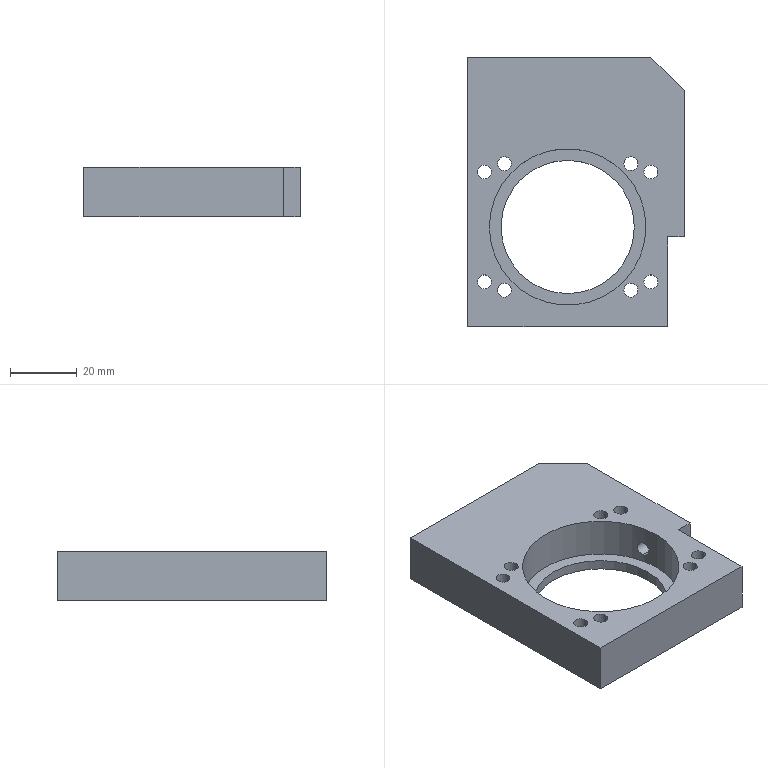Part | SolidWorks | features HoleWzd 2, MoveFace 2, MirrorStock 1 | 1 solid | 49 faces | box 65 x 81 x 15 mm | volume 49071 mm3 | cylinder 30 | plane 10 | cone 9 | commonest cylinder face diameters 4.2 x26 40 x2 47 x2
STEP:
#1=CARTESIAN_POINT('',(-24.5,27.6,-2.1));
#2=VERTEX_POINT('',#1);
#3=CARTESIAN_POINT('',(-24.5,27.6,2.1));
#4=VERTEX_POINT('',#3);
#5=CARTESIAN_POINT('',(-24.5,27.6,0.));
#6=DIRECTION('',(0.,-1.,0.));
#7=DIRECTION('',(0.,0.,-1.));
#8=AXIS2_PLACEMENT_3D('',#5,#6,#7);
#9=CIRCLE('',#8,2.1);
#10=EDGE_CURVE('',#2,#4,#9,.T.);
#11=ORIENTED_EDGE('',*,*,#10,.T.);
#12=CARTESIAN_POINT('',(-24.5,40.,2.1));
#13=VERTEX_POINT('',#12);
#14=CARTESIAN_POINT('',(-24.5,40.,2.1));
#15=DIRECTION('',(0.,1.,0.));
#16=VECTOR('',#15,1000.);
#17=LINE('',#14,#16);
#18=EDGE_CURVE('',#4,#13,#17,.T.);
#19=ORIENTED_EDGE('',*,*,#18,.T.);
#20=CARTESIAN_POINT('',(-24.5,40.,-2.1));
#21=VERTEX_POINT('',#20);
#22=CARTESIAN_POINT('',(-24.5,40.,0.));
#23=DIRECTION('',(0.,-1.,0.));
#24=DIRECTION('',(0.,0.,-1.));
#25=AXIS2_PLACEMENT_3D('',#22,#23,#24);
#26=CIRCLE('',#25,2.1);
#27=EDGE_CURVE('',#21,#13,#26,.T.);
#28=ORIENTED_EDGE('',*,*,#27,.F.);
#29=CARTESIAN_POINT('',(-24.5,40.,-2.1));
#30=DIRECTION('',(0.,1.,0.));
#31=VECTOR('',#30,1000.);
#32=LINE('',#29,#31);
#33=EDGE_CURVE('',#2,#21,#32,.T.);
#34=ORIENTED_EDGE('',*,*,#33,.F.);
#35=EDGE_LOOP('',(#11,#19,#28,#34));
#36=FACE_OUTER_BOUND('',#35,.T.);
#37=CARTESIAN_POINT('',(-24.5,40.,0.));
#38=DIRECTION('',(0.,1.,0.));
#39=DIRECTION('',(0.,0.,-1.));
#40=AXIS2_PLACEMENT_3D('',#37,#38,#39);
#41=CYLINDRICAL_SURFACE('',#40,2.1);
#42=ADVANCED_FACE('',(#36),#41,.F.);
#43=CARTESIAN_POINT('',(-24.5,26.338,0.));
#44=VERTEX_POINT('',#43);
#45=CARTESIAN_POINT('',(-24.5,27.6,-2.1));
#46=DIRECTION('',(0.,0.515,-0.8572));
#47=VECTOR('',#46,1000.);
#48=LINE('',#45,#47);
#49=EDGE_CURVE('',#44,#2,#48,.T.);
#50=ORIENTED_EDGE('',*,*,#49,.F.);
#51=CARTESIAN_POINT('',(-24.5,27.6,2.1));
#52=DIRECTION('',(0.,0.515,0.8572));
#53=VECTOR('',#52,1000.);
#54=LINE('',#51,#53);
#55=EDGE_CURVE('',#44,#4,#54,.T.);
#56=ORIENTED_EDGE('',*,*,#55,.T.);
#57=ORIENTED_EDGE('',*,*,#10,.F.);
#58=EDGE_LOOP('',(#50,#56,#57));
#59=FACE_OUTER_BOUND('',#58,.T.);
#60=CARTESIAN_POINT('',(-24.5,27.6,0.));
#61=DIRECTION('',(0.,1.,0.));
#62=DIRECTION('',(0.,0.,-1.));
#63=AXIS2_PLACEMENT_3D('',#60,#61,#62);
#64=CONICAL_SURFACE('',#63,2.1,1.03);
#65=ADVANCED_FACE('',(#59),#64,.F.);
#66=CARTESIAN_POINT('',(-5.,27.6,-2.1));
#67=VERTEX_POINT('',#66);
#68=CARTESIAN_POINT('',(-5.,27.6,2.1));
#69=VERTEX_POINT('',#68);
#70=CARTESIAN_POINT('',(-5.,27.6,0.));
#71=DIRECTION('',(0.,-1.,0.));
#72=DIRECTION('',(0.,0.,-1.));
#73=AXIS2_PLACEMENT_3D('',#70,#71,#72);
#74=CIRCLE('',#73,2.1);
#75=EDGE_CURVE('',#67,#69,#74,.T.);
#76=ORIENTED_EDGE('',*,*,#75,.T.);
#77=CARTESIAN_POINT('',(-5.,40.,2.1));
#78=VERTEX_POINT('',#77);
#79=CARTESIAN_POINT('',(-5.,40.,2.1));
#80=DIRECTION('',(0.,1.,0.));
#81=VECTOR('',#80,1000.);
#82=LINE('',#79,#81);
#83=EDGE_CURVE('',#69,#78,#82,.T.);
#84=ORIENTED_EDGE('',*,*,#83,.T.);
#85=CARTESIAN_POINT('',(-5.,40.,-2.1));
#86=VERTEX_POINT('',#85);
#87=CARTESIAN_POINT('',(-5.,40.,0.));
#88=DIRECTION('',(0.,-1.,0.));
#89=DIRECTION('',(0.,0.,-1.));
#90=AXIS2_PLACEMENT_3D('',#87,#88,#89);
#91=CIRCLE('',#90,2.1);
#92=EDGE_CURVE('',#86,#78,#91,.T.);
#93=ORIENTED_EDGE('',*,*,#92,.F.);
#94=CARTESIAN_POINT('',(-5.,40.,-2.1));
#95=DIRECTION('',(0.,1.,0.));
#96=VECTOR('',#95,1000.);
#97=LINE('',#94,#96);
#98=EDGE_CURVE('',#67,#86,#97,.T.);
#99=ORIENTED_EDGE('',*,*,#98,.F.);
#100=EDGE_LOOP('',(#76,#84,#93,#99));
#101=FACE_OUTER_BOUND('',#100,.T.);
#102=CARTESIAN_POINT('',(-5.,40.,0.));
#103=DIRECTION('',(0.,1.,0.));
#104=DIRECTION('',(0.,0.,-1.));
#105=AXIS2_PLACEMENT_3D('',#102,#103,#104);
#106=CYLINDRICAL_SURFACE('',#105,2.1);
#107=ADVANCED_FACE('',(#101),#106,.F.);
#108=CARTESIAN_POINT('',(-5.,26.338,0.));
#109=VERTEX_POINT('',#108);
#110=CARTESIAN_POINT('',(-5.,27.6,-2.1));
#111=DIRECTION('',(0.,0.515,-0.8572));
#112=VECTOR('',#111,1000.);
#113=LINE('',#110,#112);
#114=EDGE_CURVE('',#109,#67,#113,.T.);
#115=ORIENTED_EDGE('',*,*,#114,.F.);
#116=CARTESIAN_POINT('',(-5.,27.6,2.1));
#117=DIRECTION('',(0.,0.515,0.8572));
#118=VECTOR('',#117,1000.);
#119=LINE('',#116,#118);
#120=EDGE_CURVE('',#109,#69,#119,.T.);
#121=ORIENTED_EDGE('',*,*,#120,.T.);
#122=ORIENTED_EDGE('',*,*,#75,.F.);
#123=EDGE_LOOP('',(#115,#121,#122));
#124=FACE_OUTER_BOUND('',#123,.T.);
#125=CARTESIAN_POINT('',(-5.,27.6,0.));
#126=DIRECTION('',(0.,1.,0.));
#127=DIRECTION('',(0.,0.,-1.));
#128=AXIS2_PLACEMENT_3D('',#125,#126,#127);
#129=CONICAL_SURFACE('',#128,2.1,1.03);
#130=ADVANCED_FACE('',(#124),#129,.F.);
#131=CARTESIAN_POINT('',(14.5,27.6,-2.1));
#132=VERTEX_POINT('',#131);
#133=CARTESIAN_POINT('',(14.5,27.6,2.1));
#134=VERTEX_POINT('',#133);
#135=CARTESIAN_POINT('',(14.5,27.6,0.));
#136=DIRECTION('',(0.,-1.,0.));
#137=DIRECTION('',(0.,0.,-1.));
#138=AXIS2_PLACEMENT_3D('',#135,#136,#137);
#139=CIRCLE('',#138,2.1);
#140=EDGE_CURVE('',#132,#134,#139,.T.);
#141=ORIENTED_EDGE('',*,*,#140,.T.);
#142=CARTESIAN_POINT('',(14.5,40.,2.1));
#143=VERTEX_POINT('',#142);
#144=CARTESIAN_POINT('',(14.5,40.,2.1));
#145=DIRECTION('',(0.,1.,0.));
#146=VECTOR('',#145,1000.);
#147=LINE('',#144,#146);
#148=EDGE_CURVE('',#134,#143,#147,.T.);
#149=ORIENTED_EDGE('',*,*,#148,.T.);
#150=CARTESIAN_POINT('',(14.5,40.,-2.1));
#151=VERTEX_POINT('',#150);
#152=CARTESIAN_POINT('',(14.5,40.,0.));
#153=DIRECTION('',(0.,-1.,0.));
#154=DIRECTION('',(0.,0.,-1.));
#155=AXIS2_PLACEMENT_3D('',#152,#153,#154);
#156=CIRCLE('',#155,2.1);
#157=EDGE_CURVE('',#151,#143,#156,.T.);
#158=ORIENTED_EDGE('',*,*,#157,.F.);
#159=CARTESIAN_POINT('',(14.5,40.,-2.1));
#160=DIRECTION('',(0.,1.,0.));
#161=VECTOR('',#160,1000.);
#162=LINE('',#159,#161);
#163=EDGE_CURVE('',#132,#151,#162,.T.);
#164=ORIENTED_EDGE('',*,*,#163,.F.);
#165=EDGE_LOOP('',(#141,#149,#158,#164));
#166=FACE_OUTER_BOUND('',#165,.T.);
#167=CARTESIAN_POINT('',(14.5,40.,0.));
#168=DIRECTION('',(0.,1.,0.));
#169=DIRECTION('',(0.,0.,-1.));
#170=AXIS2_PLACEMENT_3D('',#167,#168,#169);
#171=CYLINDRICAL_SURFACE('',#170,2.1);
#172=ADVANCED_FACE('',(#166),#171,.F.);
#173=CARTESIAN_POINT('',(14.5,26.338,0.));
#174=VERTEX_POINT('',#173);
#175=CARTESIAN_POINT('',(14.5,27.6,-2.1));
#176=DIRECTION('',(0.,0.515,-0.8572));
#177=VECTOR('',#176,1000.);
#178=LINE('',#175,#177);
#179=EDGE_CURVE('',#174,#132,#178,.T.);
#180=ORIENTED_EDGE('',*,*,#179,.F.);
#181=CARTESIAN_POINT('',(14.5,27.6,2.1));
#182=DIRECTION('',(0.,0.515,0.8572));
#183=VECTOR('',#182,1000.);
#184=LINE('',#181,#183);
#185=EDGE_CURVE('',#174,#134,#184,.T.);
#186=ORIENTED_EDGE('',*,*,#185,.T.);
#187=ORIENTED_EDGE('',*,*,#140,.F.);
#188=EDGE_LOOP('',(#180,#186,#187));
#189=FACE_OUTER_BOUND('',#188,.T.);
#190=CARTESIAN_POINT('',(14.5,27.6,0.));
#191=DIRECTION('',(0.,1.,0.));
#192=DIRECTION('',(0.,0.,-1.));
#193=AXIS2_PLACEMENT_3D('',#190,#191,#192);
#194=CONICAL_SURFACE('',#193,2.1,1.03);
#195=ADVANCED_FACE('',(#189),#194,.F.);
#196=CARTESIAN_POINT('',(20.462,-6.,-2.1));
#197=VERTEX_POINT('',#196);
#198=CARTESIAN_POINT('',(20.1,-4.559,-1.527));
#199=VERTEX_POINT('',#198);
#200=CARTESIAN_POINT('',(20.462,-6.,-2.1));
#201=CARTESIAN_POINT('',(20.404,-5.736,-2.1));
#202=CARTESIAN_POINT('',(20.342,-5.471,-2.049));
#203=CARTESIAN_POINT('',(20.249,-5.104,-1.904));
#204=CARTESIAN_POINT('',(20.217,-4.985,-1.843));
#205=CARTESIAN_POINT('',(20.157,-4.761,-1.701));
#206=CARTESIAN_POINT('',(20.128,-4.656,-1.619));
#207=CARTESIAN_POINT('',(20.1,-4.559,-1.527));
#208=B_SPLINE_CURVE_WITH_KNOTS('',3,(#200,#201,#202,#203,#204,#205,#206,#207),.UNSPECIFIED.,.F.,.F.,(4,2,2,4),(0.008237,0.009047,0.009451,0.009856),.UNSPECIFIED.);
#209=EDGE_CURVE('',#197,#199,#208,.T.);
#210=ORIENTED_EDGE('',*,*,#209,.F.);
#211=CARTESIAN_POINT('',(32.5,-6.,-2.1));
#212=VERTEX_POINT('',#211);
#213=CARTESIAN_POINT('',(32.5,-6.,-2.1));
#214=DIRECTION('',(1.,0.,0.));
#215=VECTOR('',#214,1000.);
#216=LINE('',#213,#215);
#217=EDGE_CURVE('',#197,#212,#216,.T.);
#218=ORIENTED_EDGE('',*,*,#217,.T.);
#219=CARTESIAN_POINT('',(32.5,-6.,2.1));
#220=VERTEX_POINT('',#219);
#221=CARTESIAN_POINT('',(32.5,-6.,0.));
#222=DIRECTION('',(-1.,0.,0.));
#223=DIRECTION('',(0.,0.,1.));
#224=AXIS2_PLACEMENT_3D('',#221,#222,#223);
#225=CIRCLE('',#224,2.1);
#226=EDGE_CURVE('',#220,#212,#225,.T.);
#227=ORIENTED_EDGE('',*,*,#226,.F.);
#228=CARTESIAN_POINT('',(20.462,-6.,2.1));
#229=VERTEX_POINT('',#228);
#230=CARTESIAN_POINT('',(32.5,-6.,2.1));
#231=DIRECTION('',(1.,0.,0.));
#232=VECTOR('',#231,1000.);
#233=LINE('',#230,#232);
#234=EDGE_CURVE('',#229,#220,#233,.T.);
#235=ORIENTED_EDGE('',*,*,#234,.F.);
#236=CARTESIAN_POINT('',(20.1,-4.559,1.527));
#237=VERTEX_POINT('',#236);
#238=CARTESIAN_POINT('',(20.1,-4.559,1.527));
#239=CARTESIAN_POINT('',(20.128,-4.656,1.619));
#240=CARTESIAN_POINT('',(20.157,-4.761,1.701));
#241=CARTESIAN_POINT('',(20.217,-4.983,1.842));
#242=CARTESIAN_POINT('',(20.248,-5.102,1.903));
#243=CARTESIAN_POINT('',(20.311,-5.348,2.001));
#244=CARTESIAN_POINT('',(20.342,-5.475,2.038));
#245=CARTESIAN_POINT('',(20.403,-5.733,2.087));
#246=CARTESIAN_POINT('',(20.433,-5.867,2.1));
#247=CARTESIAN_POINT('',(20.462,-6.,2.1));
#248=B_SPLINE_CURVE_WITH_KNOTS('',3,(#238,#239,#240,#241,#242,#243,#244,#245,#246,#247),.UNSPECIFIED.,.F.,.F.,(4,2,2,2,4),(0.,0.0004052,0.0008104,0.001216,0.001621),.UNSPECIFIED.);
#249=EDGE_CURVE('',#237,#229,#248,.T.);
#250=ORIENTED_EDGE('',*,*,#249,.F.);
#251=CARTESIAN_POINT('',(20.1,-6.,0.));
#252=DIRECTION('',(-1.,0.,0.));
#253=DIRECTION('',(0.,0.,1.));
#254=AXIS2_PLACEMENT_3D('',#251,#252,#253);
#255=CIRCLE('',#254,2.1);
#256=EDGE_CURVE('',#237,#199,#255,.T.);
#257=ORIENTED_EDGE('',*,*,#256,.T.);
#258=EDGE_LOOP('',(#210,#218,#227,#235,#250,#257));
#259=FACE_OUTER_BOUND('',#258,.T.);
#260=CARTESIAN_POINT('',(32.5,-6.,0.));
#261=DIRECTION('',(1.,0.,0.));
#262=DIRECTION('',(0.,0.,1.));
#263=AXIS2_PLACEMENT_3D('',#260,#261,#262);
#264=CYLINDRICAL_SURFACE('',#263,2.1);
#265=ADVANCED_FACE('',(#259),#264,.F.);
#266=CARTESIAN_POINT('',(20.1,22.,2.1));
#267=VERTEX_POINT('',#266);
#268=CARTESIAN_POINT('',(20.1,22.,-2.1));
#269=VERTEX_POINT('',#268);
#270=CARTESIAN_POINT('',(20.1,22.,0.));
#271=DIRECTION('',(-1.,0.,0.));
#272=DIRECTION('',(0.,0.,1.));
#273=AXIS2_PLACEMENT_3D('',#270,#271,#272);
#274=CIRCLE('',#273,2.1);
#275=EDGE_CURVE('',#267,#269,#274,.T.);
#276=ORIENTED_EDGE('',*,*,#275,.T.);
#277=CARTESIAN_POINT('',(32.5,22.,-2.1));
#278=VERTEX_POINT('',#277);
#279=CARTESIAN_POINT('',(32.5,22.,-2.1));
#280=DIRECTION('',(1.,0.,0.));
#281=VECTOR('',#280,1000.);
#282=LINE('',#279,#281);
#283=EDGE_CURVE('',#269,#278,#282,.T.);
#284=ORIENTED_EDGE('',*,*,#283,.T.);
#285=CARTESIAN_POINT('',(32.5,22.,2.1));
#286=VERTEX_POINT('',#285);
#287=CARTESIAN_POINT('',(32.5,22.,0.));
#288=DIRECTION('',(-1.,0.,0.));
#289=DIRECTION('',(0.,0.,1.));
#290=AXIS2_PLACEMENT_3D('',#287,#288,#289);
#291=CIRCLE('',#290,2.1);
#292=EDGE_CURVE('',#286,#278,#291,.T.);
#293=ORIENTED_EDGE('',*,*,#292,.F.);
#294=CARTESIAN_POINT('',(32.5,22.,2.1));
#295=DIRECTION('',(1.,0.,0.));
#296=VECTOR('',#295,1000.);
#297=LINE('',#294,#296);
#298=EDGE_CURVE('',#267,#286,#297,.T.);
#299=ORIENTED_EDGE('',*,*,#298,.F.);
#300=EDGE_LOOP('',(#276,#284,#293,#299));
#301=FACE_OUTER_BOUND('',#300,.T.);
#302=CARTESIAN_POINT('',(32.5,22.,0.));
#303=DIRECTION('',(1.,0.,0.));
#304=DIRECTION('',(0.,0.,1.));
#305=AXIS2_PLACEMENT_3D('',#302,#303,#304);
#306=CYLINDRICAL_SURFACE('',#305,2.1);
#307=ADVANCED_FACE('',(#301),#306,.F.);
#308=CARTESIAN_POINT('',(18.838,22.,0.));
#309=VERTEX_POINT('',#308);
#310=CARTESIAN_POINT('',(20.1,22.,2.1));
#311=DIRECTION('',(0.515,0.,0.8572));
#312=VECTOR('',#311,1000.);
#313=LINE('',#310,#312);
#314=EDGE_CURVE('',#309,#267,#313,.T.);
#315=ORIENTED_EDGE('',*,*,#314,.F.);
#316=CARTESIAN_POINT('',(20.1,22.,-2.1));
#317=DIRECTION('',(0.515,0.,-0.8572));
#318=VECTOR('',#317,1000.);
#319=LINE('',#316,#318);
#320=EDGE_CURVE('',#309,#269,#319,.T.);
#321=ORIENTED_EDGE('',*,*,#320,.T.);
#322=ORIENTED_EDGE('',*,*,#275,.F.);
#323=EDGE_LOOP('',(#315,#321,#322));
#324=FACE_OUTER_BOUND('',#323,.T.);
#325=CARTESIAN_POINT('',(20.1,22.,0.));
#326=DIRECTION('',(1.,0.,0.));
#327=DIRECTION('',(0.,0.,1.));
#328=AXIS2_PLACEMENT_3D('',#325,#326,#327);
#329=CONICAL_SURFACE('',#328,2.1,1.03);
#330=ADVANCED_FACE('',(#324),#329,.F.);
#331=CARTESIAN_POINT('',(-19.4,8.,7.5));
#332=VERTEX_POINT('',#331);
#333=CARTESIAN_POINT('',(-23.6,8.,7.5));
#334=VERTEX_POINT('',#333);
#335=CARTESIAN_POINT('',(-21.5,8.,7.5));
#336=DIRECTION('',(0.,0.,1.));
#337=DIRECTION('',(1.,0.,0.));
#338=AXIS2_PLACEMENT_3D('',#335,#336,#337);
#339=CIRCLE('',#338,2.1);
#340=EDGE_CURVE('',#332,#334,#339,.T.);
#341=ORIENTED_EDGE('',*,*,#340,.T.);
#342=CARTESIAN_POINT('',(-23.6,8.,-7.5));
#343=VERTEX_POINT('',#342);
#344=CARTESIAN_POINT('',(-23.6,8.,-7.5));
#345=DIRECTION('',(0.,0.,-1.));
#346=VECTOR('',#345,1000.);
#347=LINE('',#344,#346);
#348=EDGE_CURVE('',#334,#343,#347,.T.);
#349=ORIENTED_EDGE('',*,*,#348,.T.);
#350=CARTESIAN_POINT('',(-19.4,8.,-7.5));
#351=VERTEX_POINT('',#350);
#352=CARTESIAN_POINT('',(-21.5,8.,-7.5));
#353=DIRECTION('',(0.,0.,1.));
#354=DIRECTION('',(1.,0.,0.));
#355=AXIS2_PLACEMENT_3D('',#352,#353,#354);
#356=CIRCLE('',#355,2.1);
#357=EDGE_CURVE('',#351,#343,#356,.T.);
#358=ORIENTED_EDGE('',*,*,#357,.F.);
#359=CARTESIAN_POINT('',(-19.4,8.,-7.5));
#360=DIRECTION('',(0.,0.,-1.));
#361=VECTOR('',#360,1000.);
#362=LINE('',#359,#361);
#363=EDGE_CURVE('',#332,#351,#362,.T.);
#364=ORIENTED_EDGE('',*,*,#363,.F.);
#365=EDGE_LOOP('',(#341,#349,#358,#364));
#366=FACE_OUTER_BOUND('',#365,.T.);
#367=CARTESIAN_POINT('',(-21.5,8.,-7.5));
#368=DIRECTION('',(0.,0.,-1.));
#369=DIRECTION('',(1.,0.,0.));
#370=AXIS2_PLACEMENT_3D('',#367,#368,#369);
#371=CYLINDRICAL_SURFACE('',#370,2.1);
#372=ADVANCED_FACE('',(#366),#371,.F.);
#373=CARTESIAN_POINT('',(-19.4,-30.,7.5));
#374=VERTEX_POINT('',#373);
#375=CARTESIAN_POINT('',(-23.6,-30.,7.5));
#376=VERTEX_POINT('',#375);
#377=CARTESIAN_POINT('',(-21.5,-30.,7.5));
#378=DIRECTION('',(0.,0.,1.));
#379=DIRECTION('',(1.,0.,0.));
#380=AXIS2_PLACEMENT_3D('',#377,#378,#379);
#381=CIRCLE('',#380,2.1);
#382=EDGE_CURVE('',#374,#376,#381,.T.);
#383=ORIENTED_EDGE('',*,*,#382,.T.);
#384=CARTESIAN_POINT('',(-23.6,-30.,-7.5));
#385=VERTEX_POINT('',#384);
#386=CARTESIAN_POINT('',(-23.6,-30.,-7.5));
#387=DIRECTION('',(0.,0.,-1.));
#388=VECTOR('',#387,1000.);
#389=LINE('',#386,#388);
#390=EDGE_CURVE('',#376,#385,#389,.T.);
#391=ORIENTED_EDGE('',*,*,#390,.T.);
#392=CARTESIAN_POINT('',(-19.4,-30.,-7.5));
#393=VERTEX_POINT('',#392);
#394=CARTESIAN_POINT('',(-21.5,-30.,-7.5));
#395=DIRECTION('',(0.,0.,1.));
#396=DIRECTION('',(1.,0.,0.));
#397=AXIS2_PLACEMENT_3D('',#394,#395,#396);
#398=CIRCLE('',#397,2.1);
#399=EDGE_CURVE('',#393,#385,#398,.T.);
#400=ORIENTED_EDGE('',*,*,#399,.F.);
#401=CARTESIAN_POINT('',(-19.4,-30.,-7.5));
#402=DIRECTION('',(0.,0.,-1.));
#403=VECTOR('',#402,1000.);
#404=LINE('',#401,#403);
#405=EDGE_CURVE('',#374,#393,#404,.T.);
#406=ORIENTED_EDGE('',*,*,#405,.F.);
#407=EDGE_LOOP('',(#383,#391,#400,#406));
#408=FACE_OUTER_BOUND('',#407,.T.);
#409=CARTESIAN_POINT('',(-21.5,-30.,-7.5));
#410=DIRECTION('',(0.,0.,-1.));
#411=DIRECTION('',(1.,0.,0.));
#412=AXIS2_PLACEMENT_3D('',#409,#410,#411);
#413=CYLINDRICAL_SURFACE('',#412,2.1);
#414=ADVANCED_FACE('',(#408),#413,.F.);
#415=CARTESIAN_POINT('',(18.6,-30.,7.5));
#416=VERTEX_POINT('',#415);
#417=CARTESIAN_POINT('',(14.4,-30.,7.5));
#418=VERTEX_POINT('',#417);
#419=CARTESIAN_POINT('',(16.5,-30.,7.5));
#420=DIRECTION('',(0.,0.,1.));
#421=DIRECTION('',(1.,0.,0.));
#422=AXIS2_PLACEMENT_3D('',#419,#420,#421);
#423=CIRCLE('',#422,2.1);
#424=EDGE_CURVE('',#416,#418,#423,.T.);
#425=ORIENTED_EDGE('',*,*,#424,.T.);
#426=CARTESIAN_POINT('',(14.4,-30.,-7.5));
#427=VERTEX_POINT('',#426);
#428=CARTESIAN_POINT('',(14.4,-30.,-7.5));
#429=DIRECTION('',(0.,0.,-1.));
#430=VECTOR('',#429,1000.);
#431=LINE('',#428,#430);
#432=EDGE_CURVE('',#418,#427,#431,.T.);
#433=ORIENTED_EDGE('',*,*,#432,.T.);
#434=CARTESIAN_POINT('',(18.6,-30.,-7.5));
#435=VERTEX_POINT('',#434);
#436=CARTESIAN_POINT('',(16.5,-30.,-7.5));
#437=DIRECTION('',(0.,0.,1.));
#438=DIRECTION('',(1.,0.,0.));
#439=AXIS2_PLACEMENT_3D('',#436,#437,#438);
#440=CIRCLE('',#439,2.1);
#441=EDGE_CURVE('',#435,#427,#440,.T.);
#442=ORIENTED_EDGE('',*,*,#441,.F.);
#443=CARTESIAN_POINT('',(18.6,-30.,-7.5));
#444=DIRECTION('',(0.,0.,-1.));
#445=VECTOR('',#444,1000.);
#446=LINE('',#443,#445);
#447=EDGE_CURVE('',#416,#435,#446,.T.);
#448=ORIENTED_EDGE('',*,*,#447,.F.);
#449=EDGE_LOOP('',(#425,#433,#442,#448));
#450=FACE_OUTER_BOUND('',#449,.T.);
#451=CARTESIAN_POINT('',(16.5,-30.,-7.5));
#452=DIRECTION('',(0.,0.,-1.));
#453=DIRECTION('',(1.,0.,0.));
#454=AXIS2_PLACEMENT_3D('',#451,#452,#453);
#455=CYLINDRICAL_SURFACE('',#454,2.1);
#456=ADVANCED_FACE('',(#450),#455,.F.);
#457=CARTESIAN_POINT('',(18.6,8.,7.5));
#458=VERTEX_POINT('',#457);
#459=CARTESIAN_POINT('',(14.4,8.,7.5));
#460=VERTEX_POINT('',#459);
#461=CARTESIAN_POINT('',(16.5,8.,7.5));
#462=DIRECTION('',(0.,0.,1.));
#463=DIRECTION('',(1.,0.,0.));
#464=AXIS2_PLACEMENT_3D('',#461,#462,#463);
#465=CIRCLE('',#464,2.1);
#466=EDGE_CURVE('',#458,#460,#465,.T.);
#467=ORIENTED_EDGE('',*,*,#466,.T.);
#468=CARTESIAN_POINT('',(14.4,8.,-7.5));
#469=VERTEX_POINT('',#468);
#470=CARTESIAN_POINT('',(14.4,8.,-7.5));
#471=DIRECTION('',(0.,0.,-1.));
#472=VECTOR('',#471,1000.);
#473=LINE('',#470,#472);
#474=EDGE_CURVE('',#460,#469,#473,.T.);
#475=ORIENTED_EDGE('',*,*,#474,.T.);
#476=CARTESIAN_POINT('',(18.6,8.,-7.5));
#477=VERTEX_POINT('',#476);
#478=CARTESIAN_POINT('',(16.5,8.,-7.5));
#479=DIRECTION('',(0.,0.,1.));
#480=DIRECTION('',(1.,0.,0.));
#481=AXIS2_PLACEMENT_3D('',#478,#479,#480);
#482=CIRCLE('',#481,2.1);
#483=EDGE_CURVE('',#477,#469,#482,.T.);
#484=ORIENTED_EDGE('',*,*,#483,.F.);
#485=CARTESIAN_POINT('',(18.6,8.,-7.5));
#486=DIRECTION('',(0.,0.,-1.));
#487=VECTOR('',#486,1000.);
#488=LINE('',#485,#487);
#489=EDGE_CURVE('',#458,#477,#488,.T.);
#490=ORIENTED_EDGE('',*,*,#489,.F.);
#491=EDGE_LOOP('',(#467,#475,#484,#490));
#492=FACE_OUTER_BOUND('',#491,.T.);
#493=CARTESIAN_POINT('',(16.5,8.,-7.5));
#494=DIRECTION('',(0.,0.,-1.));
#495=DIRECTION('',(1.,0.,0.));
#496=AXIS2_PLACEMENT_3D('',#493,#494,#495);
#497=CYLINDRICAL_SURFACE('',#496,2.1);
#498=ADVANCED_FACE('',(#492),#497,.F.);
#499=CARTESIAN_POINT('',(20.4,5.5,-7.5));
#500=VERTEX_POINT('',#499);
#501=CARTESIAN_POINT('',(24.6,5.5,-7.5));
#502=VERTEX_POINT('',#501);
#503=CARTESIAN_POINT('',(22.5,5.5,-7.5));
#504=DIRECTION('',(0.,0.,-1.));
#505=DIRECTION('',(-1.,0.,0.));
#506=AXIS2_PLACEMENT_3D('',#503,#504,#505);
#507=CIRCLE('',#506,2.1);
#508=EDGE_CURVE('',#500,#502,#507,.T.);
#509=ORIENTED_EDGE('',*,*,#508,.T.);
#510=CARTESIAN_POINT('',(24.6,5.5,7.5));
#511=VERTEX_POINT('',#510);
#512=CARTESIAN_POINT('',(24.6,5.5,7.5));
#513=DIRECTION('',(0.,0.,1.));
#514=VECTOR('',#513,1000.);
#515=LINE('',#512,#514);
#516=EDGE_CURVE('',#502,#511,#515,.T.);
#517=ORIENTED_EDGE('',*,*,#516,.T.);
#518=CARTESIAN_POINT('',(20.4,5.5,7.5));
#519=VERTEX_POINT('',#518);
#520=CARTESIAN_POINT('',(22.5,5.5,7.5));
#521=DIRECTION('',(0.,0.,-1.));
#522=DIRECTION('',(-1.,0.,0.));
#523=AXIS2_PLACEMENT_3D('',#520,#521,#522);
#524=CIRCLE('',#523,2.1);
#525=EDGE_CURVE('',#519,#511,#524,.T.);
#526=ORIENTED_EDGE('',*,*,#525,.F.);
#527=CARTESIAN_POINT('',(20.4,5.5,7.5));
#528=DIRECTION('',(0.,0.,1.));
#529=VECTOR('',#528,1000.);
#530=LINE('',#527,#529);
#531=EDGE_CURVE('',#500,#519,#530,.T.);
#532=ORIENTED_EDGE('',*,*,#531,.F.);
#533=EDGE_LOOP('',(#509,#517,#526,#532));
#534=FACE_OUTER_BOUND('',#533,.T.);
#535=CARTESIAN_POINT('',(22.5,5.5,7.5));
#536=DIRECTION('',(0.,0.,1.));
#537=DIRECTION('',(-1.,0.,0.));
#538=AXIS2_PLACEMENT_3D('',#535,#536,#537);
#539=CYLINDRICAL_SURFACE('',#538,2.1);
#540=ADVANCED_FACE('',(#534),#539,.F.);
#541=CARTESIAN_POINT('',(20.4,-27.5,-7.5));
#542=VERTEX_POINT('',#541);
#543=CARTESIAN_POINT('',(24.6,-27.5,-7.5));
#544=VERTEX_POINT('',#543);
#545=CARTESIAN_POINT('',(22.5,-27.5,-7.5));
#546=DIRECTION('',(0.,0.,-1.));
#547=DIRECTION('',(-1.,0.,0.));
#548=AXIS2_PLACEMENT_3D('',#545,#546,#547);
#549=CIRCLE('',#548,2.1);
#550=EDGE_CURVE('',#542,#544,#549,.T.);
#551=ORIENTED_EDGE('',*,*,#550,.T.);
#552=CARTESIAN_POINT('',(24.6,-27.5,7.5));
#553=VERTEX_POINT('',#552);
#554=CARTESIAN_POINT('',(24.6,-27.5,7.5));
#555=DIRECTION('',(0.,0.,1.));
#556=VECTOR('',#555,1000.);
#557=LINE('',#554,#556);
#558=EDGE_CURVE('',#544,#553,#557,.T.);
#559=ORIENTED_EDGE('',*,*,#558,.T.);
#560=CARTESIAN_POINT('',(20.4,-27.5,7.5));
#561=VERTEX_POINT('',#560);
#562=CARTESIAN_POINT('',(22.5,-27.5,7.5));
#563=DIRECTION('',(0.,0.,-1.));
#564=DIRECTION('',(-1.,0.,0.));
#565=AXIS2_PLACEMENT_3D('',#562,#563,#564);
#566=CIRCLE('',#565,2.1);
#567=EDGE_CURVE('',#561,#553,#566,.T.);
#568=ORIENTED_EDGE('',*,*,#567,.F.);
#569=CARTESIAN_POINT('',(20.4,-27.5,7.5));
#570=DIRECTION('',(0.,0.,1.));
#571=VECTOR('',#570,1000.);
#572=LINE('',#569,#571);
#573=EDGE_CURVE('',#542,#561,#572,.T.);
#574=ORIENTED_EDGE('',*,*,#573,.F.);
#575=EDGE_LOOP('',(#551,#559,#568,#574));
#576=FACE_OUTER_BOUND('',#575,.T.);
#577=CARTESIAN_POINT('',(22.5,-27.5,7.5));
#578=DIRECTION('',(0.,0.,1.));
#579=DIRECTION('',(-1.,0.,0.));
#580=AXIS2_PLACEMENT_3D('',#577,#578,#579);
#581=CYLINDRICAL_SURFACE('',#580,2.1);
#582=ADVANCED_FACE('',(#576),#581,.F.);
#583=CARTESIAN_POINT('',(-29.6,-27.5,-7.5));
#584=VERTEX_POINT('',#583);
#585=CARTESIAN_POINT('',(-25.4,-27.5,-7.5));
#586=VERTEX_POINT('',#585);
#587=CARTESIAN_POINT('',(-27.5,-27.5,-7.5));
#588=DIRECTION('',(0.,0.,-1.));
#589=DIRECTION('',(-1.,0.,0.));
#590=AXIS2_PLACEMENT_3D('',#587,#588,#589);
#591=CIRCLE('',#590,2.1);
#592=EDGE_CURVE('',#584,#586,#591,.T.);
#593=ORIENTED_EDGE('',*,*,#592,.T.);
#594=CARTESIAN_POINT('',(-25.4,-27.5,7.5));
#595=VERTEX_POINT('',#594);
#596=CARTESIAN_POINT('',(-25.4,-27.5,7.5));
#597=DIRECTION('',(0.,0.,1.));
#598=VECTOR('',#597,1000.);
#599=LINE('',#596,#598);
#600=EDGE_CURVE('',#586,#595,#599,.T.);
#601=ORIENTED_EDGE('',*,*,#600,.T.);
#602=CARTESIAN_POINT('',(-29.6,-27.5,7.5));
#603=VERTEX_POINT('',#602);
#604=CARTESIAN_POINT('',(-27.5,-27.5,7.5));
#605=DIRECTION('',(0.,0.,-1.));
#606=DIRECTION('',(-1.,0.,0.));
#607=AXIS2_PLACEMENT_3D('',#604,#605,#606);
#608=CIRCLE('',#607,2.1);
#609=EDGE_CURVE('',#603,#595,#608,.T.);
#610=ORIENTED_EDGE('',*,*,#609,.F.);
#611=CARTESIAN_POINT('',(-29.6,-27.5,7.5));
#612=DIRECTION('',(0.,0.,1.));
#613=VECTOR('',#612,1000.);
#614=LINE('',#611,#613);
#615=EDGE_CURVE('',#584,#603,#614,.T.);
#616=ORIENTED_EDGE('',*,*,#615,.F.);
#617=EDGE_LOOP('',(#593,#601,#610,#616));
#618=FACE_OUTER_BOUND('',#617,.T.);
#619=CARTESIAN_POINT('',(-27.5,-27.5,7.5));
#620=DIRECTION('',(0.,0.,1.));
#621=DIRECTION('',(-1.,0.,0.));
#622=AXIS2_PLACEMENT_3D('',#619,#620,#621);
#623=CYLINDRICAL_SURFACE('',#622,2.1);
#624=ADVANCED_FACE('',(#618),#623,.F.);
#625=CARTESIAN_POINT('',(-29.6,5.5,-7.5));
#626=VERTEX_POINT('',#625);
#627=CARTESIAN_POINT('',(-25.4,5.5,-7.5));
#628=VERTEX_POINT('',#627);
#629=CARTESIAN_POINT('',(-27.5,5.5,-7.5));
#630=DIRECTION('',(0.,0.,-1.));
#631=DIRECTION('',(-1.,0.,0.));
#632=AXIS2_PLACEMENT_3D('',#629,#630,#631);
#633=CIRCLE('',#632,2.1);
#634=EDGE_CURVE('',#626,#628,#633,.T.);
#635=ORIENTED_EDGE('',*,*,#634,.T.);
#636=CARTESIAN_POINT('',(-25.4,5.5,7.5));
#637=VERTEX_POINT('',#636);
#638=CARTESIAN_POINT('',(-25.4,5.5,7.5));
#639=DIRECTION('',(0.,0.,1.));
#640=VECTOR('',#639,1000.);
#641=LINE('',#638,#640);
#642=EDGE_CURVE('',#628,#637,#641,.T.);
#643=ORIENTED_EDGE('',*,*,#642,.T.);
#644=CARTESIAN_POINT('',(-29.6,5.5,7.5));
#645=VERTEX_POINT('',#644);
#646=CARTESIAN_POINT('',(-27.5,5.5,7.5));
#647=DIRECTION('',(0.,0.,-1.));
#648=DIRECTION('',(-1.,0.,0.));
#649=AXIS2_PLACEMENT_3D('',#646,#647,#648);
#650=CIRCLE('',#649,2.1);
#651=EDGE_CURVE('',#645,#637,#650,.T.);
#652=ORIENTED_EDGE('',*,*,#651,.F.);
#653=CARTESIAN_POINT('',(-29.6,5.5,7.5));
#654=DIRECTION('',(0.,0.,1.));
#655=VECTOR('',#654,1000.);
#656=LINE('',#653,#655);
#657=EDGE_CURVE('',#626,#645,#656,.T.);
#658=ORIENTED_EDGE('',*,*,#657,.F.);
#659=EDGE_LOOP('',(#635,#643,#652,#658));
#660=FACE_OUTER_BOUND('',#659,.T.);
#661=CARTESIAN_POINT('',(-27.5,5.5,7.5));
#662=DIRECTION('',(0.,0.,1.));
#663=DIRECTION('',(-1.,0.,0.));
#664=AXIS2_PLACEMENT_3D('',#661,#662,#663);
#665=CYLINDRICAL_SURFACE('',#664,2.1);
#666=ADVANCED_FACE('',(#660),#665,.F.);
#667=CARTESIAN_POINT('',(-22.5,-11.,-7.5));
#668=VERTEX_POINT('',#667);
#669=CARTESIAN_POINT('',(17.5,-11.,-7.5));
#670=VERTEX_POINT('',#669);
#671=CARTESIAN_POINT('',(-2.5,-11.,-7.5));
#672=DIRECTION('',(0.,0.,-1.));
#673=DIRECTION('',(-1.,0.,0.));
#674=AXIS2_PLACEMENT_3D('',#671,#672,#673);
#675=CIRCLE('',#674,20.);
#676=EDGE_CURVE('',#668,#670,#675,.T.);
#677=ORIENTED_EDGE('',*,*,#676,.T.);
#678=CARTESIAN_POINT('',(17.5,-11.,-4.5));
#679=VERTEX_POINT('',#678);
#680=CARTESIAN_POINT('',(17.5,-11.,-7.5));
#681=DIRECTION('',(0.,0.,1.));
#682=VECTOR('',#681,1000.);
#683=LINE('',#680,#682);
#684=EDGE_CURVE('',#670,#679,#683,.T.);
#685=ORIENTED_EDGE('',*,*,#684,.T.);
#686=CARTESIAN_POINT('',(-22.5,-11.,-4.5));
#687=VERTEX_POINT('',#686);
#688=CARTESIAN_POINT('',(-2.5,-11.,-4.5));
#689=DIRECTION('',(0.,0.,-1.));
#690=DIRECTION('',(-1.,0.,0.));
#691=AXIS2_PLACEMENT_3D('',#688,#689,#690);
#692=CIRCLE('',#691,20.);
#693=EDGE_CURVE('',#687,#679,#692,.T.);
#694=ORIENTED_EDGE('',*,*,#693,.F.);
#695=CARTESIAN_POINT('',(-22.5,-11.,-7.5));
#696=DIRECTION('',(0.,0.,1.));
#697=VECTOR('',#696,1000.);
#698=LINE('',#695,#697);
#699=EDGE_CURVE('',#668,#687,#698,.T.);
#700=ORIENTED_EDGE('',*,*,#699,.F.);
#701=EDGE_LOOP('',(#677,#685,#694,#700));
#702=FACE_OUTER_BOUND('',#701,.T.);
#703=CARTESIAN_POINT('',(-2.5,-11.,-7.5));
#704=DIRECTION('',(0.,0.,1.));
#705=DIRECTION('',(-1.,0.,0.));
#706=AXIS2_PLACEMENT_3D('',#703,#704,#705);
#707=CYLINDRICAL_SURFACE('',#706,20.);
#708=ADVANCED_FACE('',(#702),#707,.F.);
#709=CARTESIAN_POINT('',(20.1,-4.559,-1.527));
#710=CARTESIAN_POINT('',(20.08,-4.488,-1.415));
#711=CARTESIAN_POINT('',(20.061,-4.424,-1.295));
#712=CARTESIAN_POINT('',(20.029,-4.314,-1.051));
#713=CARTESIAN_POINT('',(20.015,-4.268,-0.9255));
#714=CARTESIAN_POINT('',(19.982,-4.157,-0.5411));
#715=CARTESIAN_POINT('',(19.969,-4.117,-0.2687));
#716=CARTESIAN_POINT('',(19.969,-4.117,0.1339));
#717=CARTESIAN_POINT('',(19.972,-4.127,0.2677));
#718=CARTESIAN_POINT('',(19.984,-4.165,0.5343));
#719=CARTESIAN_POINT('',(19.993,-4.193,0.6679));
#720=CARTESIAN_POINT('',(20.027,-4.306,1.055));
#721=CARTESIAN_POINT('',(20.059,-4.417,1.3));
#722=CARTESIAN_POINT('',(20.1,-4.559,1.527));
#723=B_SPLINE_CURVE_WITH_KNOTS('',3,(#709,#710,#711,#712,#713,#714,#715,#716,#717,#718,#719,#720,#721,#722),.UNSPECIFIED.,.F.,.F.,(4,2,2,2,2,2,4),(0.0007393,0.001141,0.001544,0.002348,0.00275,0.003152,0.003956),.UNSPECIFIED.);
#724=EDGE_CURVE('',#199,#237,#723,.T.);
#725=ORIENTED_EDGE('',*,*,#724,.T.);
#726=ORIENTED_EDGE('',*,*,#249,.T.);
#727=CARTESIAN_POINT('',(20.462,-6.,2.1));
#728=CARTESIAN_POINT('',(20.491,-6.135,2.1));
#729=CARTESIAN_POINT('',(20.519,-6.27,2.087));
#730=CARTESIAN_POINT('',(20.573,-6.536,2.035));
#731=CARTESIAN_POINT('',(20.598,-6.669,1.995));
#732=CARTESIAN_POINT('',(20.644,-6.921,1.892));
#733=CARTESIAN_POINT('',(20.665,-7.042,1.829));
#734=CARTESIAN_POINT('',(20.703,-7.271,1.677));
#735=CARTESIAN_POINT('',(20.72,-7.379,1.589));
#736=CARTESIAN_POINT('',(20.764,-7.672,1.3));
#737=CARTESIAN_POINT('',(20.786,-7.831,1.065));
#738=CARTESIAN_POINT('',(20.807,-7.99,0.6837));
#739=CARTESIAN_POINT('',(20.812,-8.032,0.5492));
#740=CARTESIAN_POINT('',(20.819,-8.086,0.2775));
#741=CARTESIAN_POINT('',(20.82,-8.1,0.1403));
#742=CARTESIAN_POINT('',(20.82,-8.1,-0.1369));
#743=CARTESIAN_POINT('',(20.819,-8.086,-0.277));
#744=CARTESIAN_POINT('',(20.812,-8.032,-0.5476));
#745=CARTESIAN_POINT('',(20.807,-7.992,-0.6797));
#746=CARTESIAN_POINT('',(20.793,-7.884,-0.9373));
#747=CARTESIAN_POINT('',(20.784,-7.819,-1.059));
#748=CARTESIAN_POINT('',(20.762,-7.665,-1.287));
#749=CARTESIAN_POINT('',(20.749,-7.576,-1.395));
#750=CARTESIAN_POINT('',(20.72,-7.38,-1.589));
#751=CARTESIAN_POINT('',(20.703,-7.273,-1.676));
#752=CARTESIAN_POINT('',(20.665,-7.045,-1.827));
#753=CARTESIAN_POINT('',(20.644,-6.921,-1.892));
#754=CARTESIAN_POINT('',(20.575,-6.543,-2.047));
#755=CARTESIAN_POINT('',(20.521,-6.27,-2.1));
#756=CARTESIAN_POINT('',(20.462,-6.,-2.1));
#757=B_SPLINE_CURVE_WITH_KNOTS('',3,(#727,#728,#729,#730,#731,#732,#733,#734,#735,#736,#737,#738,#739,#740,#741,#742,#743,#744,#745,#746,#747,#748,#749,#750,#751,#752,#753,#754,#755,#756),.UNSPECIFIED.,.F.,.F.,(4,2,2,2,2,2,2,2,2,2,2,2,2,2,4),(0.001621,0.002034,0.002448,0.002861,0.003275,0.004102,0.004516,0.004929,0.005343,0.005756,0.00617,0.006583,0.006997,0.00741,0.008237),.UNSPECIFIED.);
#758=EDGE_CURVE('',#229,#197,#757,.T.);
#759=ORIENTED_EDGE('',*,*,#758,.T.);
#760=ORIENTED_EDGE('',*,*,#209,.T.);
#761=EDGE_LOOP('',(#725,#726,#759,#760));
#762=FACE_BOUND('',#761,.T.);
#763=CARTESIAN_POINT('',(21.,-11.,-4.5));
#764=VERTEX_POINT('',#763);
#765=CARTESIAN_POINT('',(-26.,-11.,-4.5));
#766=VERTEX_POINT('',#765);
#767=CARTESIAN_POINT('',(-2.5,-11.,-4.5));
#768=DIRECTION('',(0.,0.,1.));
#769=DIRECTION('',(1.,0.,0.));
#770=AXIS2_PLACEMENT_3D('',#767,#768,#769);
#771=CIRCLE('',#770,23.5);
#772=EDGE_CURVE('',#764,#766,#771,.T.);
#773=ORIENTED_EDGE('',*,*,#772,.F.);
#774=CARTESIAN_POINT('',(21.,-11.,7.5));
#775=VERTEX_POINT('',#774);
#776=CARTESIAN_POINT('',(21.,-11.,-4.5));
#777=DIRECTION('',(0.,0.,1.));
#778=VECTOR('',#777,1000.);
#779=LINE('',#776,#778);
#780=EDGE_CURVE('',#764,#775,#779,.T.);
#781=ORIENTED_EDGE('',*,*,#780,.T.);
#782=CARTESIAN_POINT('',(-26.,-11.,7.5));
#783=VERTEX_POINT('',#782);
#784=CARTESIAN_POINT('',(-2.5,-11.,7.5));
#785=DIRECTION('',(0.,0.,1.));
#786=DIRECTION('',(1.,0.,0.));
#787=AXIS2_PLACEMENT_3D('',#784,#785,#786);
#788=CIRCLE('',#787,23.5);
#789=EDGE_CURVE('',#775,#783,#788,.T.);
#790=ORIENTED_EDGE('',*,*,#789,.T.);
#791=CARTESIAN_POINT('',(-26.,-11.,-4.5));
#792=DIRECTION('',(0.,0.,1.));
#793=VECTOR('',#792,1000.);
#794=LINE('',#791,#793);
#795=EDGE_CURVE('',#766,#783,#794,.T.);
#796=ORIENTED_EDGE('',*,*,#795,.F.);
#797=EDGE_LOOP('',(#773,#781,#790,#796));
#798=FACE_OUTER_BOUND('',#797,.T.);
#799=CARTESIAN_POINT('',(-2.5,-11.,-4.5));
#800=DIRECTION('',(0.,0.,1.));
#801=DIRECTION('',(-1.,0.,0.));
#802=AXIS2_PLACEMENT_3D('',#799,#800,#801);
#803=CYLINDRICAL_SURFACE('',#802,23.5);
#804=ADVANCED_FACE('',(#762,#798),#803,.F.);
#805=ORIENTED_EDGE('',*,*,#226,.T.);
#806=CARTESIAN_POINT('',(32.5,-6.,0.));
#807=DIRECTION('',(-1.,0.,0.));
#808=DIRECTION('',(0.,0.,1.));
#809=AXIS2_PLACEMENT_3D('',#806,#807,#808);
#810=CIRCLE('',#809,2.1);
#811=EDGE_CURVE('',#212,#220,#810,.T.);
#812=ORIENTED_EDGE('',*,*,#811,.T.);
#813=EDGE_LOOP('',(#805,#812));
#814=FACE_BOUND('',#813,.T.);
#815=ORIENTED_EDGE('',*,*,#292,.T.);
#816=CARTESIAN_POINT('',(32.5,22.,0.));
#817=DIRECTION('',(-1.,0.,0.));
#818=DIRECTION('',(0.,0.,1.));
#819=AXIS2_PLACEMENT_3D('',#816,#817,#818);
#820=CIRCLE('',#819,2.1);
#821=EDGE_CURVE('',#278,#286,#820,.T.);
#822=ORIENTED_EDGE('',*,*,#821,.T.);
#823=EDGE_LOOP('',(#815,#822));
#824=FACE_BOUND('',#823,.T.);
#825=CARTESIAN_POINT('',(32.5,-14.,7.5));
#826=VERTEX_POINT('',#825);
#827=CARTESIAN_POINT('',(32.5,30.,7.5));
#828=VERTEX_POINT('',#827);
#829=CARTESIAN_POINT('',(32.5,-41.,7.5));
#830=DIRECTION('',(0.,1.,0.));
#831=VECTOR('',#830,1000.);
#832=LINE('',#829,#831);
#833=EDGE_CURVE('',#826,#828,#832,.T.);
#834=ORIENTED_EDGE('',*,*,#833,.F.);
#835=CARTESIAN_POINT('',(32.5,-14.,-7.5));
#836=VERTEX_POINT('',#835);
#837=CARTESIAN_POINT('',(32.5,-14.,7.5));
#838=DIRECTION('',(0.,0.,-1.));
#839=VECTOR('',#838,1000.);
#840=LINE('',#837,#839);
#841=EDGE_CURVE('',#826,#836,#840,.T.);
#842=ORIENTED_EDGE('',*,*,#841,.T.);
#843=CARTESIAN_POINT('',(32.5,30.,-7.5));
#844=VERTEX_POINT('',#843);
#845=CARTESIAN_POINT('',(32.5,-41.,-7.5));
#846=DIRECTION('',(0.,1.,0.));
#847=VECTOR('',#846,1000.);
#848=LINE('',#845,#847);
#849=EDGE_CURVE('',#836,#844,#848,.T.);
#850=ORIENTED_EDGE('',*,*,#849,.T.);
#851=CARTESIAN_POINT('',(32.5,30.,-7.5));
#852=DIRECTION('',(0.,0.,-1.));
#853=VECTOR('',#852,1000.);
#854=LINE('',#851,#853);
#855=EDGE_CURVE('',#828,#844,#854,.T.);
#856=ORIENTED_EDGE('',*,*,#855,.F.);
#857=EDGE_LOOP('',(#834,#842,#850,#856));
#858=FACE_OUTER_BOUND('',#857,.T.);
#859=CARTESIAN_POINT('',(32.5,-41.,-7.5));
#860=DIRECTION('',(-1.,0.,0.));
#861=DIRECTION('',(0.,0.,-1.));
#862=AXIS2_PLACEMENT_3D('',#859,#860,#861);
#863=PLANE('',#862);
#864=ADVANCED_FACE('',(#814,#824,#858),#863,.F.);
#865=ORIENTED_EDGE('',*,*,#27,.T.);
#866=CARTESIAN_POINT('',(-24.5,40.,0.));
#867=DIRECTION('',(0.,-1.,0.));
#868=DIRECTION('',(0.,0.,-1.));
#869=AXIS2_PLACEMENT_3D('',#866,#867,#868);
#870=CIRCLE('',#869,2.1);
#871=EDGE_CURVE('',#13,#21,#870,.T.);
#872=ORIENTED_EDGE('',*,*,#871,.T.);
#873=EDGE_LOOP('',(#865,#872));
#874=FACE_BOUND('',#873,.T.);
#875=ORIENTED_EDGE('',*,*,#92,.T.);
#876=CARTESIAN_POINT('',(-5.,40.,0.));
#877=DIRECTION('',(0.,-1.,0.));
#878=DIRECTION('',(0.,0.,-1.));
#879=AXIS2_PLACEMENT_3D('',#876,#877,#878);
#880=CIRCLE('',#879,2.1);
#881=EDGE_CURVE('',#78,#86,#880,.T.);
#882=ORIENTED_EDGE('',*,*,#881,.T.);
#883=EDGE_LOOP('',(#875,#882));
#884=FACE_BOUND('',#883,.T.);
#885=ORIENTED_EDGE('',*,*,#157,.T.);
#886=CARTESIAN_POINT('',(14.5,40.,0.));
#887=DIRECTION('',(0.,-1.,0.));
#888=DIRECTION('',(0.,0.,-1.));
#889=AXIS2_PLACEMENT_3D('',#886,#887,#888);
#890=CIRCLE('',#889,2.1);
#891=EDGE_CURVE('',#143,#151,#890,.T.);
#892=ORIENTED_EDGE('',*,*,#891,.T.);
#893=EDGE_LOOP('',(#885,#892));
#894=FACE_BOUND('',#893,.T.);
#895=CARTESIAN_POINT('',(22.5,40.,-7.5));
#896=VERTEX_POINT('',#895);
#897=CARTESIAN_POINT('',(-32.5,40.,-7.5));
#898=VERTEX_POINT('',#897);
#899=CARTESIAN_POINT('',(-32.5,40.,-7.5));
#900=DIRECTION('',(-1.,0.,0.));
#901=VECTOR('',#900,1000.);
#902=LINE('',#899,#901);
#903=EDGE_CURVE('',#896,#898,#902,.T.);
#904=ORIENTED_EDGE('',*,*,#903,.T.);
#905=CARTESIAN_POINT('',(-32.5,40.,7.5));
#906=VERTEX_POINT('',#905);
#907=CARTESIAN_POINT('',(-32.5,40.,-7.5));
#908=DIRECTION('',(0.,0.,1.));
#909=VECTOR('',#908,1000.);
#910=LINE('',#907,#909);
#911=EDGE_CURVE('',#898,#906,#910,.T.);
#912=ORIENTED_EDGE('',*,*,#911,.T.);
#913=CARTESIAN_POINT('',(22.5,40.,7.5));
#914=VERTEX_POINT('',#913);
#915=CARTESIAN_POINT('',(-32.5,40.,7.5));
#916=DIRECTION('',(-1.,0.,0.));
#917=VECTOR('',#916,1000.);
#918=LINE('',#915,#917);
#919=EDGE_CURVE('',#914,#906,#918,.T.);
#920=ORIENTED_EDGE('',*,*,#919,.F.);
#921=CARTESIAN_POINT('',(22.5,40.,-7.5));
#922=DIRECTION('',(0.,0.,1.));
#923=VECTOR('',#922,1000.);
#924=LINE('',#921,#923);
#925=EDGE_CURVE('',#896,#914,#924,.T.);
#926=ORIENTED_EDGE('',*,*,#925,.F.);
#927=EDGE_LOOP('',(#904,#912,#920,#926));
#928=FACE_OUTER_BOUND('',#927,.T.);
#929=CARTESIAN_POINT('',(-32.5,40.,-7.5));
#930=DIRECTION('',(0.,-1.,0.));
#931=DIRECTION('',(0.,0.,1.));
#932=AXIS2_PLACEMENT_3D('',#929,#930,#931);
#933=PLANE('',#932);
#934=ADVANCED_FACE('',(#874,#884,#894,#928),#933,.F.);
#935=CARTESIAN_POINT('',(-32.5,-41.,7.5));
#936=VERTEX_POINT('',#935);
#937=CARTESIAN_POINT('',(-32.5,-41.,7.5));
#938=DIRECTION('',(0.,-1.,0.));
#939=VECTOR('',#938,1000.);
#940=LINE('',#937,#939);
#941=EDGE_CURVE('',#906,#936,#940,.T.);
#942=ORIENTED_EDGE('',*,*,#941,.F.);
#943=ORIENTED_EDGE('',*,*,#911,.F.);
#944=CARTESIAN_POINT('',(-32.5,-41.,-7.5));
#945=VERTEX_POINT('',#944);
#946=CARTESIAN_POINT('',(-32.5,-41.,-7.5));
#947=DIRECTION('',(0.,-1.,0.));
#948=VECTOR('',#947,1000.);
#949=LINE('',#946,#948);
#950=EDGE_CURVE('',#898,#945,#949,.T.);
#951=ORIENTED_EDGE('',*,*,#950,.T.);
#952=CARTESIAN_POINT('',(-32.5,-41.,-7.5));
#953=DIRECTION('',(0.,0.,1.));
#954=VECTOR('',#953,1000.);
#955=LINE('',#952,#954);
#956=EDGE_CURVE('',#945,#936,#955,.T.);
#957=ORIENTED_EDGE('',*,*,#956,.T.);
#958=EDGE_LOOP('',(#942,#943,#951,#957));
#959=FACE_OUTER_BOUND('',#958,.T.);
#960=CARTESIAN_POINT('',(-32.5,-41.,-7.5));
#961=DIRECTION('',(1.,0.,0.));
#962=DIRECTION('',(0.,0.,1.));
#963=AXIS2_PLACEMENT_3D('',#960,#961,#962);
#964=PLANE('',#963);
#965=ADVANCED_FACE('',(#959),#964,.F.);
#966=CARTESIAN_POINT('',(27.5,-41.,7.5));
#967=VERTEX_POINT('',#966);
#968=CARTESIAN_POINT('',(-32.5,-41.,7.5));
#969=DIRECTION('',(1.,0.,0.));
#970=VECTOR('',#969,1000.);
#971=LINE('',#968,#970);
#972=EDGE_CURVE('',#936,#967,#971,.T.);
#973=ORIENTED_EDGE('',*,*,#972,.F.);
#974=ORIENTED_EDGE('',*,*,#956,.F.);
#975=CARTESIAN_POINT('',(27.5,-41.,-7.5));
#976=VERTEX_POINT('',#975);
#977=CARTESIAN_POINT('',(-32.5,-41.,-7.5));
#978=DIRECTION('',(1.,0.,0.));
#979=VECTOR('',#978,1000.);
#980=LINE('',#977,#979);
#981=EDGE_CURVE('',#945,#976,#980,.T.);
#982=ORIENTED_EDGE('',*,*,#981,.T.);
#983=CARTESIAN_POINT('',(27.5,-41.,7.5));
#984=DIRECTION('',(0.,0.,-1.));
#985=VECTOR('',#984,1000.);
#986=LINE('',#983,#985);
#987=EDGE_CURVE('',#967,#976,#986,.T.);
#988=ORIENTED_EDGE('',*,*,#987,.F.);
#989=EDGE_LOOP('',(#973,#974,#982,#988));
#990=FACE_OUTER_BOUND('',#989,.T.);
#991=CARTESIAN_POINT('',(-32.5,-41.,-7.5));
#992=DIRECTION('',(0.,1.,0.));
#993=DIRECTION('',(0.,0.,-1.));
#994=AXIS2_PLACEMENT_3D('',#991,#992,#993);
#995=PLANE('',#994);
#996=ADVANCED_FACE('',(#990),#995,.F.);
#997=ORIENTED_EDGE('',*,*,#357,.T.);
#998=CARTESIAN_POINT('',(-21.5,8.,-7.5));
#999=DIRECTION('',(0.,0.,1.));
#1000=DIRECTION('',(1.,0.,0.));
#1001=AXIS2_PLACEMENT_3D('',#998,#999,#1000);
#1002=CIRCLE('',#1001,2.1);
#1003=EDGE_CURVE('',#343,#351,#1002,.T.);
#1004=ORIENTED_EDGE('',*,*,#1003,.T.);
#1005=EDGE_LOOP('',(#997,#1004));
#1006=FACE_BOUND('',#1005,.T.);
#1007=ORIENTED_EDGE('',*,*,#399,.T.);
#1008=CARTESIAN_POINT('',(-21.5,-30.,-7.5));
#1009=DIRECTION('',(0.,0.,1.));
#1010=DIRECTION('',(1.,0.,0.));
#1011=AXIS2_PLACEMENT_3D('',#1008,#1009,#1010);
#1012=CIRCLE('',#1011,2.1);
#1013=EDGE_CURVE('',#385,#393,#1012,.T.);
#1014=ORIENTED_EDGE('',*,*,#1013,.T.);
#1015=EDGE_LOOP('',(#1007,#1014));
#1016=FACE_BOUND('',#1015,.T.);
#1017=ORIENTED_EDGE('',*,*,#441,.T.);
#1018=CARTESIAN_POINT('',(16.5,-30.,-7.5));
#1019=DIRECTION('',(0.,0.,1.));
#1020=DIRECTION('',(1.,0.,0.));
#1021=AXIS2_PLACEMENT_3D('',#1018,#1019,#1020);
#1022=CIRCLE('',#1021,2.1);
#1023=EDGE_CURVE('',#427,#435,#1022,.T.);
#1024=ORIENTED_EDGE('',*,*,#1023,.T.);
#1025=EDGE_LOOP('',(#1017,#1024));
#1026=FACE_BOUND('',#1025,.T.);
#1027=ORIENTED_EDGE('',*,*,#483,.T.);
#1028=CARTESIAN_POINT('',(16.5,8.,-7.5));
#1029=DIRECTION('',(0.,0.,1.));
#1030=DIRECTION('',(1.,0.,0.));
#1031=AXIS2_PLACEMENT_3D('',#1028,#1029,#1030);
#1032=CIRCLE('',#1031,2.1);
#1033=EDGE_CURVE('',#469,#477,#1032,.T.);
#1034=ORIENTED_EDGE('',*,*,#1033,.T.);
#1035=EDGE_LOOP('',(#1027,#1034));
#1036=FACE_BOUND('',#1035,.T.);
#1037=ORIENTED_EDGE('',*,*,#508,.F.);
#1038=CARTESIAN_POINT('',(22.5,5.5,-7.5));
#1039=DIRECTION('',(0.,0.,-1.));
#1040=DIRECTION('',(-1.,0.,0.));
#1041=AXIS2_PLACEMENT_3D('',#1038,#1039,#1040);
#1042=CIRCLE('',#1041,2.1);
#1043=EDGE_CURVE('',#502,#500,#1042,.T.);
#1044=ORIENTED_EDGE('',*,*,#1043,.F.);
#1045=EDGE_LOOP('',(#1037,#1044));
#1046=FACE_BOUND('',#1045,.T.);
#1047=ORIENTED_EDGE('',*,*,#550,.F.);
#1048=CARTESIAN_POINT('',(22.5,-27.5,-7.5));
#1049=DIRECTION('',(0.,0.,-1.));
#1050=DIRECTION('',(-1.,0.,0.));
#1051=AXIS2_PLACEMENT_3D('',#1048,#1049,#1050);
#1052=CIRCLE('',#1051,2.1);
#1053=EDGE_CURVE('',#544,#542,#1052,.T.);
#1054=ORIENTED_EDGE('',*,*,#1053,.F.);
#1055=EDGE_LOOP('',(#1047,#1054));
#1056=FACE_BOUND('',#1055,.T.);
#1057=ORIENTED_EDGE('',*,*,#592,.F.);
#1058=CARTESIAN_POINT('',(-27.5,-27.5,-7.5));
#1059=DIRECTION('',(0.,0.,-1.));
#1060=DIRECTION('',(-1.,0.,0.));
#1061=AXIS2_PLACEMENT_3D('',#1058,#1059,#1060);
#1062=CIRCLE('',#1061,2.1);
#1063=EDGE_CURVE('',#586,#584,#1062,.T.);
#1064=ORIENTED_EDGE('',*,*,#1063,.F.);
#1065=EDGE_LOOP('',(#1057,#1064));
#1066=FACE_BOUND('',#1065,.T.);
#1067=ORIENTED_EDGE('',*,*,#634,.F.);
#1068=CARTESIAN_POINT('',(-27.5,5.5,-7.5));
#1069=DIRECTION('',(0.,0.,-1.));
#1070=DIRECTION('',(-1.,0.,0.));
#1071=AXIS2_PLACEMENT_3D('',#1068,#1069,#1070);
#1072=CIRCLE('',#1071,2.1);
#1073=EDGE_CURVE('',#628,#626,#1072,.T.);
#1074=ORIENTED_EDGE('',*,*,#1073,.F.);
#1075=EDGE_LOOP('',(#1067,#1074));
#1076=FACE_BOUND('',#1075,.T.);
#1077=ORIENTED_EDGE('',*,*,#676,.F.);
#1078=CARTESIAN_POINT('',(-2.5,-11.,-7.5));
#1079=DIRECTION('',(0.,0.,-1.));
#1080=DIRECTION('',(-1.,0.,0.));
#1081=AXIS2_PLACEMENT_3D('',#1078,#1079,#1080);
#1082=CIRCLE('',#1081,20.);
#1083=EDGE_CURVE('',#670,#668,#1082,.T.);
#1084=ORIENTED_EDGE('',*,*,#1083,.F.);
#1085=EDGE_LOOP('',(#1077,#1084));
#1086=FACE_BOUND('',#1085,.T.);
#1087=ORIENTED_EDGE('',*,*,#849,.F.);
#1088=CARTESIAN_POINT('',(27.5,-14.,-7.5));
#1089=VERTEX_POINT('',#1088);
#1090=CARTESIAN_POINT('',(27.5,-14.,-7.5));
#1091=DIRECTION('',(-1.,0.,0.));
#1092=VECTOR('',#1091,1000.);
#1093=LINE('',#1090,#1092);
#1094=EDGE_CURVE('',#836,#1089,#1093,.T.);
#1095=ORIENTED_EDGE('',*,*,#1094,.T.);
#1096=CARTESIAN_POINT('',(27.5,-41.,-7.5));
#1097=DIRECTION('',(0.,-1.,0.));
#1098=VECTOR('',#1097,1000.);
#1099=LINE('',#1096,#1098);
#1100=EDGE_CURVE('',#1089,#976,#1099,.T.);
#1101=ORIENTED_EDGE('',*,*,#1100,.T.);
#1102=ORIENTED_EDGE('',*,*,#981,.F.);
#1103=ORIENTED_EDGE('',*,*,#950,.F.);
#1104=ORIENTED_EDGE('',*,*,#903,.F.);
#1105=CARTESIAN_POINT('',(22.5,40.,-7.5));
#1106=DIRECTION('',(-0.7071,0.7071,0.));
#1107=VECTOR('',#1106,1000.);
#1108=LINE('',#1105,#1107);
#1109=EDGE_CURVE('',#844,#896,#1108,.T.);
#1110=ORIENTED_EDGE('',*,*,#1109,.F.);
#1111=EDGE_LOOP('',(#1087,#1095,#1101,#1102,#1103,#1104,#1110));
#1112=FACE_OUTER_BOUND('',#1111,.T.);
#1113=CARTESIAN_POINT('',(0.,0.,-7.5));
#1114=DIRECTION('',(0.,0.,1.));
#1115=DIRECTION('',(-1.,0.,0.));
#1116=AXIS2_PLACEMENT_3D('',#1113,#1114,#1115);
#1117=PLANE('',#1116);
#1118=ADVANCED_FACE('',(#1006,#1016,#1026,#1036,#1046,#1056,#1066,#1076,#1086,#1112),#1117,.F.);
#1119=ORIENTED_EDGE('',*,*,#340,.F.);
#1120=CARTESIAN_POINT('',(-21.5,8.,7.5));
#1121=DIRECTION('',(0.,0.,1.));
#1122=DIRECTION('',(1.,0.,0.));
#1123=AXIS2_PLACEMENT_3D('',#1120,#1121,#1122);
#1124=CIRCLE('',#1123,2.1);
#1125=EDGE_CURVE('',#334,#332,#1124,.T.);
#1126=ORIENTED_EDGE('',*,*,#1125,.F.);
#1127=EDGE_LOOP('',(#1119,#1126));
#1128=FACE_BOUND('',#1127,.T.);
#1129=ORIENTED_EDGE('',*,*,#382,.F.);
#1130=CARTESIAN_POINT('',(-21.5,-30.,7.5));
#1131=DIRECTION('',(0.,0.,1.));
#1132=DIRECTION('',(1.,0.,0.));
#1133=AXIS2_PLACEMENT_3D('',#1130,#1131,#1132);
#1134=CIRCLE('',#1133,2.1);
#1135=EDGE_CURVE('',#376,#374,#1134,.T.);
#1136=ORIENTED_EDGE('',*,*,#1135,.F.);
#1137=EDGE_LOOP('',(#1129,#1136));
#1138=FACE_BOUND('',#1137,.T.);
#1139=ORIENTED_EDGE('',*,*,#424,.F.);
#1140=CARTESIAN_POINT('',(16.5,-30.,7.5));
#1141=DIRECTION('',(0.,0.,1.));
#1142=DIRECTION('',(1.,0.,0.));
#1143=AXIS2_PLACEMENT_3D('',#1140,#1141,#1142);
#1144=CIRCLE('',#1143,2.1);
#1145=EDGE_CURVE('',#418,#416,#1144,.T.);
#1146=ORIENTED_EDGE('',*,*,#1145,.F.);
#1147=EDGE_LOOP('',(#1139,#1146));
#1148=FACE_BOUND('',#1147,.T.);
#1149=ORIENTED_EDGE('',*,*,#466,.F.);
#1150=CARTESIAN_POINT('',(16.5,8.,7.5));
#1151=DIRECTION('',(0.,0.,1.));
#1152=DIRECTION('',(1.,0.,0.));
#1153=AXIS2_PLACEMENT_3D('',#1150,#1151,#1152);
#1154=CIRCLE('',#1153,2.1);
#1155=EDGE_CURVE('',#460,#458,#1154,.T.);
#1156=ORIENTED_EDGE('',*,*,#1155,.F.);
#1157=EDGE_LOOP('',(#1149,#1156));
#1158=FACE_BOUND('',#1157,.T.);
#1159=ORIENTED_EDGE('',*,*,#525,.T.);
#1160=CARTESIAN_POINT('',(22.5,5.5,7.5));
#1161=DIRECTION('',(0.,0.,-1.));
#1162=DIRECTION('',(-1.,0.,0.));
#1163=AXIS2_PLACEMENT_3D('',#1160,#1161,#1162);
#1164=CIRCLE('',#1163,2.1);
#1165=EDGE_CURVE('',#511,#519,#1164,.T.);
#1166=ORIENTED_EDGE('',*,*,#1165,.T.);
#1167=EDGE_LOOP('',(#1159,#1166));
#1168=FACE_BOUND('',#1167,.T.);
#1169=ORIENTED_EDGE('',*,*,#567,.T.);
#1170=CARTESIAN_POINT('',(22.5,-27.5,7.5));
#1171=DIRECTION('',(0.,0.,-1.));
#1172=DIRECTION('',(-1.,0.,0.));
#1173=AXIS2_PLACEMENT_3D('',#1170,#1171,#1172);
#1174=CIRCLE('',#1173,2.1);
#1175=EDGE_CURVE('',#553,#561,#1174,.T.);
#1176=ORIENTED_EDGE('',*,*,#1175,.T.);
#1177=EDGE_LOOP('',(#1169,#1176));
#1178=FACE_BOUND('',#1177,.T.);
#1179=ORIENTED_EDGE('',*,*,#609,.T.);
#1180=CARTESIAN_POINT('',(-27.5,-27.5,7.5));
#1181=DIRECTION('',(0.,0.,-1.));
#1182=DIRECTION('',(-1.,0.,0.));
#1183=AXIS2_PLACEMENT_3D('',#1180,#1181,#1182);
#1184=CIRCLE('',#1183,2.1);
#1185=EDGE_CURVE('',#595,#603,#1184,.T.);
#1186=ORIENTED_EDGE('',*,*,#1185,.T.);
#1187=EDGE_LOOP('',(#1179,#1186));
#1188=FACE_BOUND('',#1187,.T.);
#1189=ORIENTED_EDGE('',*,*,#651,.T.);
#1190=CARTESIAN_POINT('',(-27.5,5.5,7.5));
#1191=DIRECTION('',(0.,0.,-1.));
#1192=DIRECTION('',(-1.,0.,0.));
#1193=AXIS2_PLACEMENT_3D('',#1190,#1191,#1192);
#1194=CIRCLE('',#1193,2.1);
#1195=EDGE_CURVE('',#637,#645,#1194,.T.);
#1196=ORIENTED_EDGE('',*,*,#1195,.T.);
#1197=EDGE_LOOP('',(#1189,#1196));
#1198=FACE_BOUND('',#1197,.T.);
#1199=ORIENTED_EDGE('',*,*,#919,.T.);
#1200=ORIENTED_EDGE('',*,*,#941,.T.);
#1201=ORIENTED_EDGE('',*,*,#972,.T.);
#1202=CARTESIAN_POINT('',(27.5,-14.,7.5));
#1203=VERTEX_POINT('',#1202);
#1204=CARTESIAN_POINT('',(27.5,-41.,7.5));
#1205=DIRECTION('',(0.,-1.,0.));
#1206=VECTOR('',#1205,1000.);
#1207=LINE('',#1204,#1206);
#1208=EDGE_CURVE('',#1203,#967,#1207,.T.);
#1209=ORIENTED_EDGE('',*,*,#1208,.F.);
#1210=CARTESIAN_POINT('',(27.5,-14.,7.5));
#1211=DIRECTION('',(-1.,0.,0.));
#1212=VECTOR('',#1211,1000.);
#1213=LINE('',#1210,#1212);
#1214=EDGE_CURVE('',#826,#1203,#1213,.T.);
#1215=ORIENTED_EDGE('',*,*,#1214,.F.);
#1216=ORIENTED_EDGE('',*,*,#833,.T.);
#1217=CARTESIAN_POINT('',(31.25,31.25,7.5));
#1218=DIRECTION('',(0.7071,-0.7071,0.));
#1219=VECTOR('',#1218,1000.);
#1220=LINE('',#1217,#1219);
#1221=EDGE_CURVE('',#914,#828,#1220,.T.);
#1222=ORIENTED_EDGE('',*,*,#1221,.F.);
#1223=EDGE_LOOP('',(#1199,#1200,#1201,#1209,#1215,#1216,#1222));
#1224=FACE_OUTER_BOUND('',#1223,.T.);
#1225=CARTESIAN_POINT('',(-2.5,-11.,7.5));
#1226=DIRECTION('',(0.,0.,1.));
#1227=DIRECTION('',(1.,0.,0.));
#1228=AXIS2_PLACEMENT_3D('',#1225,#1226,#1227);
#1229=CIRCLE('',#1228,23.5);
#1230=EDGE_CURVE('',#783,#775,#1229,.T.);
#1231=ORIENTED_EDGE('',*,*,#1230,.F.);
#1232=ORIENTED_EDGE('',*,*,#789,.F.);
#1233=EDGE_LOOP('',(#1231,#1232));
#1234=FACE_BOUND('',#1233,.T.);
#1235=CARTESIAN_POINT('',(0.,0.,7.5));
#1236=DIRECTION('',(0.,0.,1.));
#1237=DIRECTION('',(-1.,0.,0.));
#1238=AXIS2_PLACEMENT_3D('',#1235,#1236,#1237);
#1239=PLANE('',#1238);
#1240=ADVANCED_FACE('',(#1128,#1138,#1148,#1158,#1168,#1178,#1188,#1198,#1224,#1234),#1239,.T.);
#1241=ORIENTED_EDGE('',*,*,#780,.F.);
#1242=CARTESIAN_POINT('',(-2.5,-11.,-4.5));
#1243=DIRECTION('',(0.,0.,1.));
#1244=DIRECTION('',(1.,0.,0.));
#1245=AXIS2_PLACEMENT_3D('',#1242,#1243,#1244);
#1246=CIRCLE('',#1245,23.5);
#1247=EDGE_CURVE('',#766,#764,#1246,.T.);
#1248=ORIENTED_EDGE('',*,*,#1247,.F.);
#1249=ORIENTED_EDGE('',*,*,#795,.T.);
#1250=ORIENTED_EDGE('',*,*,#1230,.T.);
#1251=EDGE_LOOP('',(#1241,#1248,#1249,#1250));
#1252=FACE_OUTER_BOUND('',#1251,.T.);
#1253=CARTESIAN_POINT('',(-2.5,-11.,-4.5));
#1254=DIRECTION('',(0.,0.,1.));
#1255=DIRECTION('',(-1.,0.,0.));
#1256=AXIS2_PLACEMENT_3D('',#1253,#1254,#1255);
#1257=CYLINDRICAL_SURFACE('',#1256,23.5);
#1258=ADVANCED_FACE('',(#1252),#1257,.F.);
#1259=ORIENTED_EDGE('',*,*,#693,.T.);
#1260=CARTESIAN_POINT('',(-2.5,-11.,-4.5));
#1261=DIRECTION('',(0.,0.,-1.));
#1262=DIRECTION('',(-1.,0.,0.));
#1263=AXIS2_PLACEMENT_3D('',#1260,#1261,#1262);
#1264=CIRCLE('',#1263,20.);
#1265=EDGE_CURVE('',#679,#687,#1264,.T.);
#1266=ORIENTED_EDGE('',*,*,#1265,.T.);
#1267=EDGE_LOOP('',(#1259,#1266));
#1268=FACE_BOUND('',#1267,.T.);
#1269=ORIENTED_EDGE('',*,*,#1247,.T.);
#1270=ORIENTED_EDGE('',*,*,#772,.T.);
#1271=EDGE_LOOP('',(#1269,#1270));
#1272=FACE_OUTER_BOUND('',#1271,.T.);
#1273=CARTESIAN_POINT('',(-2.5,-11.,-4.5));
#1274=DIRECTION('',(0.,0.,-1.));
#1275=DIRECTION('',(1.,0.,0.));
#1276=AXIS2_PLACEMENT_3D('',#1273,#1274,#1275);
#1277=PLANE('',#1276);
#1278=ADVANCED_FACE('',(#1268,#1272),#1277,.F.);
#1279=ORIENTED_EDGE('',*,*,#684,.F.);
#1280=ORIENTED_EDGE('',*,*,#1083,.T.);
#1281=ORIENTED_EDGE('',*,*,#699,.T.);
#1282=ORIENTED_EDGE('',*,*,#1265,.F.);
#1283=EDGE_LOOP('',(#1279,#1280,#1281,#1282));
#1284=FACE_OUTER_BOUND('',#1283,.T.);
#1285=CARTESIAN_POINT('',(-2.5,-11.,-7.5));
#1286=DIRECTION('',(0.,0.,1.));
#1287=DIRECTION('',(-1.,0.,0.));
#1288=AXIS2_PLACEMENT_3D('',#1285,#1286,#1287);
#1289=CYLINDRICAL_SURFACE('',#1288,20.);
#1290=ADVANCED_FACE('',(#1284),#1289,.F.);
#1291=ORIENTED_EDGE('',*,*,#1100,.F.);
#1292=CARTESIAN_POINT('',(27.5,-14.,7.5));
#1293=DIRECTION('',(0.,0.,-1.));
#1294=VECTOR('',#1293,1000.);
#1295=LINE('',#1292,#1294);
#1296=EDGE_CURVE('',#1203,#1089,#1295,.T.);
#1297=ORIENTED_EDGE('',*,*,#1296,.F.);
#1298=ORIENTED_EDGE('',*,*,#1208,.T.);
#1299=ORIENTED_EDGE('',*,*,#987,.T.);
#1300=EDGE_LOOP('',(#1291,#1297,#1298,#1299));
#1301=FACE_OUTER_BOUND('',#1300,.T.);
#1302=CARTESIAN_POINT('',(27.5,-41.,7.5));
#1303=DIRECTION('',(-1.,0.,0.));
#1304=DIRECTION('',(0.,0.,-1.));
#1305=AXIS2_PLACEMENT_3D('',#1302,#1303,#1304);
#1306=PLANE('',#1305);
#1307=ADVANCED_FACE('',(#1301),#1306,.F.);
#1308=ORIENTED_EDGE('',*,*,#1094,.F.);
#1309=ORIENTED_EDGE('',*,*,#841,.F.);
#1310=ORIENTED_EDGE('',*,*,#1214,.T.);
#1311=ORIENTED_EDGE('',*,*,#1296,.T.);
#1312=EDGE_LOOP('',(#1308,#1309,#1310,#1311));
#1313=FACE_OUTER_BOUND('',#1312,.T.);
#1314=CARTESIAN_POINT('',(27.5,-14.,7.5));
#1315=DIRECTION('',(0.,1.,0.));
#1316=DIRECTION('',(0.,0.,-1.));
#1317=AXIS2_PLACEMENT_3D('',#1314,#1315,#1316);
#1318=PLANE('',#1317);
#1319=ADVANCED_FACE('',(#1313),#1318,.F.);
#1320=ORIENTED_EDGE('',*,*,#642,.F.);
#1321=ORIENTED_EDGE('',*,*,#1073,.T.);
#1322=ORIENTED_EDGE('',*,*,#657,.T.);
#1323=ORIENTED_EDGE('',*,*,#1195,.F.);
#1324=EDGE_LOOP('',(#1320,#1321,#1322,#1323));
#1325=FACE_OUTER_BOUND('',#1324,.T.);
#1326=CARTESIAN_POINT('',(-27.5,5.5,7.5));
#1327=DIRECTION('',(0.,0.,1.));
#1328=DIRECTION('',(-1.,0.,0.));
#1329=AXIS2_PLACEMENT_3D('',#1326,#1327,#1328);
#1330=CYLINDRICAL_SURFACE('',#1329,2.1);
#1331=ADVANCED_FACE('',(#1325),#1330,.F.);
#1332=ORIENTED_EDGE('',*,*,#600,.F.);
#1333=ORIENTED_EDGE('',*,*,#1063,.T.);
#1334=ORIENTED_EDGE('',*,*,#615,.T.);
#1335=ORIENTED_EDGE('',*,*,#1185,.F.);
#1336=EDGE_LOOP('',(#1332,#1333,#1334,#1335));
#1337=FACE_OUTER_BOUND('',#1336,.T.);
#1338=CARTESIAN_POINT('',(-27.5,-27.5,7.5));
#1339=DIRECTION('',(0.,0.,1.));
#1340=DIRECTION('',(-1.,0.,0.));
#1341=AXIS2_PLACEMENT_3D('',#1338,#1339,#1340);
#1342=CYLINDRICAL_SURFACE('',#1341,2.1);
#1343=ADVANCED_FACE('',(#1337),#1342,.F.);
#1344=ORIENTED_EDGE('',*,*,#558,.F.);
#1345=ORIENTED_EDGE('',*,*,#1053,.T.);
#1346=ORIENTED_EDGE('',*,*,#573,.T.);
#1347=ORIENTED_EDGE('',*,*,#1175,.F.);
#1348=EDGE_LOOP('',(#1344,#1345,#1346,#1347));
#1349=FACE_OUTER_BOUND('',#1348,.T.);
#1350=CARTESIAN_POINT('',(22.5,-27.5,7.5));
#1351=DIRECTION('',(0.,0.,1.));
#1352=DIRECTION('',(-1.,0.,0.));
#1353=AXIS2_PLACEMENT_3D('',#1350,#1351,#1352);
#1354=CYLINDRICAL_SURFACE('',#1353,2.1);
#1355=ADVANCED_FACE('',(#1349),#1354,.F.);
#1356=ORIENTED_EDGE('',*,*,#516,.F.);
#1357=ORIENTED_EDGE('',*,*,#1043,.T.);
#1358=ORIENTED_EDGE('',*,*,#531,.T.);
#1359=ORIENTED_EDGE('',*,*,#1165,.F.);
#1360=EDGE_LOOP('',(#1356,#1357,#1358,#1359));
#1361=FACE_OUTER_BOUND('',#1360,.T.);
#1362=CARTESIAN_POINT('',(22.5,5.5,7.5));
#1363=DIRECTION('',(0.,0.,1.));
#1364=DIRECTION('',(-1.,0.,0.));
#1365=AXIS2_PLACEMENT_3D('',#1362,#1363,#1364);
#1366=CYLINDRICAL_SURFACE('',#1365,2.1);
#1367=ADVANCED_FACE('',(#1361),#1366,.F.);
#1368=ORIENTED_EDGE('',*,*,#474,.F.);
#1369=ORIENTED_EDGE('',*,*,#1155,.T.);
#1370=ORIENTED_EDGE('',*,*,#489,.T.);
#1371=ORIENTED_EDGE('',*,*,#1033,.F.);
#1372=EDGE_LOOP('',(#1368,#1369,#1370,#1371));
#1373=FACE_OUTER_BOUND('',#1372,.T.);
#1374=CARTESIAN_POINT('',(16.5,8.,-7.5));
#1375=DIRECTION('',(0.,0.,-1.));
#1376=DIRECTION('',(1.,0.,0.));
#1377=AXIS2_PLACEMENT_3D('',#1374,#1375,#1376);
#1378=CYLINDRICAL_SURFACE('',#1377,2.1);
#1379=ADVANCED_FACE('',(#1373),#1378,.F.);
#1380=ORIENTED_EDGE('',*,*,#432,.F.);
#1381=ORIENTED_EDGE('',*,*,#1145,.T.);
#1382=ORIENTED_EDGE('',*,*,#447,.T.);
#1383=ORIENTED_EDGE('',*,*,#1023,.F.);
#1384=EDGE_LOOP('',(#1380,#1381,#1382,#1383));
#1385=FACE_OUTER_BOUND('',#1384,.T.);
#1386=CARTESIAN_POINT('',(16.5,-30.,-7.5));
#1387=DIRECTION('',(0.,0.,-1.));
#1388=DIRECTION('',(1.,0.,0.));
#1389=AXIS2_PLACEMENT_3D('',#1386,#1387,#1388);
#1390=CYLINDRICAL_SURFACE('',#1389,2.1);
#1391=ADVANCED_FACE('',(#1385),#1390,.F.);
#1392=ORIENTED_EDGE('',*,*,#390,.F.);
#1393=ORIENTED_EDGE('',*,*,#1135,.T.);
#1394=ORIENTED_EDGE('',*,*,#405,.T.);
#1395=ORIENTED_EDGE('',*,*,#1013,.F.);
#1396=EDGE_LOOP('',(#1392,#1393,#1394,#1395));
#1397=FACE_OUTER_BOUND('',#1396,.T.);
#1398=CARTESIAN_POINT('',(-21.5,-30.,-7.5));
#1399=DIRECTION('',(0.,0.,-1.));
#1400=DIRECTION('',(1.,0.,0.));
#1401=AXIS2_PLACEMENT_3D('',#1398,#1399,#1400);
#1402=CYLINDRICAL_SURFACE('',#1401,2.1);
#1403=ADVANCED_FACE('',(#1397),#1402,.F.);
#1404=ORIENTED_EDGE('',*,*,#348,.F.);
#1405=ORIENTED_EDGE('',*,*,#1125,.T.);
#1406=ORIENTED_EDGE('',*,*,#363,.T.);
#1407=ORIENTED_EDGE('',*,*,#1003,.F.);
#1408=EDGE_LOOP('',(#1404,#1405,#1406,#1407));
#1409=FACE_OUTER_BOUND('',#1408,.T.);
#1410=CARTESIAN_POINT('',(-21.5,8.,-7.5));
#1411=DIRECTION('',(0.,0.,-1.));
#1412=DIRECTION('',(1.,0.,0.));
#1413=AXIS2_PLACEMENT_3D('',#1410,#1411,#1412);
#1414=CYLINDRICAL_SURFACE('',#1413,2.1);
#1415=ADVANCED_FACE('',(#1409),#1414,.F.);
#1416=ORIENTED_EDGE('',*,*,#320,.F.);
#1417=ORIENTED_EDGE('',*,*,#314,.T.);
#1418=CARTESIAN_POINT('',(20.1,22.,0.));
#1419=DIRECTION('',(-1.,0.,0.));
#1420=DIRECTION('',(0.,0.,1.));
#1421=AXIS2_PLACEMENT_3D('',#1418,#1419,#1420);
#1422=CIRCLE('',#1421,2.1);
#1423=EDGE_CURVE('',#269,#267,#1422,.T.);
#1424=ORIENTED_EDGE('',*,*,#1423,.F.);
#1425=EDGE_LOOP('',(#1416,#1417,#1424));
#1426=FACE_OUTER_BOUND('',#1425,.T.);
#1427=CARTESIAN_POINT('',(20.1,22.,0.));
#1428=DIRECTION('',(1.,0.,0.));
#1429=DIRECTION('',(0.,0.,1.));
#1430=AXIS2_PLACEMENT_3D('',#1427,#1428,#1429);
#1431=CONICAL_SURFACE('',#1430,2.1,1.03);
#1432=ADVANCED_FACE('',(#1426),#1431,.F.);
#1433=ORIENTED_EDGE('',*,*,#283,.F.);
#1434=ORIENTED_EDGE('',*,*,#1423,.T.);
#1435=ORIENTED_EDGE('',*,*,#298,.T.);
#1436=ORIENTED_EDGE('',*,*,#821,.F.);
#1437=EDGE_LOOP('',(#1433,#1434,#1435,#1436));
#1438=FACE_OUTER_BOUND('',#1437,.T.);
#1439=CARTESIAN_POINT('',(32.5,22.,0.));
#1440=DIRECTION('',(1.,0.,0.));
#1441=DIRECTION('',(0.,0.,1.));
#1442=AXIS2_PLACEMENT_3D('',#1439,#1440,#1441);
#1443=CYLINDRICAL_SURFACE('',#1442,2.1);
#1444=ADVANCED_FACE('',(#1438),#1443,.F.);
#1445=ORIENTED_EDGE('',*,*,#724,.F.);
#1446=ORIENTED_EDGE('',*,*,#256,.F.);
#1447=EDGE_LOOP('',(#1445,#1446));
#1448=FACE_OUTER_BOUND('',#1447,.T.);
#1449=CARTESIAN_POINT('',(20.1,-6.,0.));
#1450=DIRECTION('',(1.,0.,0.));
#1451=DIRECTION('',(0.,0.,1.));
#1452=AXIS2_PLACEMENT_3D('',#1449,#1450,#1451);
#1453=CONICAL_SURFACE('',#1452,2.1,1.03);
#1454=ADVANCED_FACE('',(#1448),#1453,.F.);
#1455=ORIENTED_EDGE('',*,*,#217,.F.);
#1456=ORIENTED_EDGE('',*,*,#758,.F.);
#1457=ORIENTED_EDGE('',*,*,#234,.T.);
#1458=ORIENTED_EDGE('',*,*,#811,.F.);
#1459=EDGE_LOOP('',(#1455,#1456,#1457,#1458));
#1460=FACE_OUTER_BOUND('',#1459,.T.);
#1461=CARTESIAN_POINT('',(32.5,-6.,0.));
#1462=DIRECTION('',(1.,0.,0.));
#1463=DIRECTION('',(0.,0.,1.));
#1464=AXIS2_PLACEMENT_3D('',#1461,#1462,#1463);
#1465=CYLINDRICAL_SURFACE('',#1464,2.1);
#1466=ADVANCED_FACE('',(#1460),#1465,.F.);
#1467=ORIENTED_EDGE('',*,*,#1109,.T.);
#1468=ORIENTED_EDGE('',*,*,#925,.T.);
#1469=ORIENTED_EDGE('',*,*,#1221,.T.);
#1470=ORIENTED_EDGE('',*,*,#855,.T.);
#1471=EDGE_LOOP('',(#1467,#1468,#1469,#1470));
#1472=FACE_OUTER_BOUND('',#1471,.T.);
#1473=CARTESIAN_POINT('',(22.5,40.,-7.5));
#1474=DIRECTION('',(-0.7071,-0.7071,0.));
#1475=DIRECTION('',(0.,0.,1.));
#1476=AXIS2_PLACEMENT_3D('',#1473,#1474,#1475);
#1477=PLANE('',#1476);
#1478=ADVANCED_FACE('',(#1472),#1477,.F.);
#1479=ORIENTED_EDGE('',*,*,#185,.F.);
#1480=ORIENTED_EDGE('',*,*,#179,.T.);
#1481=CARTESIAN_POINT('',(14.5,27.6,0.));
#1482=DIRECTION('',(0.,-1.,0.));
#1483=DIRECTION('',(0.,0.,-1.));
#1484=AXIS2_PLACEMENT_3D('',#1481,#1482,#1483);
#1485=CIRCLE('',#1484,2.1);
#1486=EDGE_CURVE('',#134,#132,#1485,.T.);
#1487=ORIENTED_EDGE('',*,*,#1486,.F.);
#1488=EDGE_LOOP('',(#1479,#1480,#1487));
#1489=FACE_OUTER_BOUND('',#1488,.T.);
#1490=CARTESIAN_POINT('',(14.5,27.6,0.));
#1491=DIRECTION('',(0.,1.,0.));
#1492=DIRECTION('',(0.,0.,-1.));
#1493=AXIS2_PLACEMENT_3D('',#1490,#1491,#1492);
#1494=CONICAL_SURFACE('',#1493,2.1,1.03);
#1495=ADVANCED_FACE('',(#1489),#1494,.F.);
#1496=ORIENTED_EDGE('',*,*,#148,.F.);
#1497=ORIENTED_EDGE('',*,*,#1486,.T.);
#1498=ORIENTED_EDGE('',*,*,#163,.T.);
#1499=ORIENTED_EDGE('',*,*,#891,.F.);
#1500=EDGE_LOOP('',(#1496,#1497,#1498,#1499));
#1501=FACE_OUTER_BOUND('',#1500,.T.);
#1502=CARTESIAN_POINT('',(14.5,40.,0.));
#1503=DIRECTION('',(0.,1.,0.));
#1504=DIRECTION('',(0.,0.,-1.));
#1505=AXIS2_PLACEMENT_3D('',#1502,#1503,#1504);
#1506=CYLINDRICAL_SURFACE('',#1505,2.1);
#1507=ADVANCED_FACE('',(#1501),#1506,.F.);
#1508=ORIENTED_EDGE('',*,*,#120,.F.);
#1509=ORIENTED_EDGE('',*,*,#114,.T.);
#1510=CARTESIAN_POINT('',(-5.,27.6,0.));
#1511=DIRECTION('',(0.,-1.,0.));
#1512=DIRECTION('',(0.,0.,-1.));
#1513=AXIS2_PLACEMENT_3D('',#1510,#1511,#1512);
#1514=CIRCLE('',#1513,2.1);
#1515=EDGE_CURVE('',#69,#67,#1514,.T.);
#1516=ORIENTED_EDGE('',*,*,#1515,.F.);
#1517=EDGE_LOOP('',(#1508,#1509,#1516));
#1518=FACE_OUTER_BOUND('',#1517,.T.);
#1519=CARTESIAN_POINT('',(-5.,27.6,0.));
#1520=DIRECTION('',(0.,1.,0.));
#1521=DIRECTION('',(0.,0.,-1.));
#1522=AXIS2_PLACEMENT_3D('',#1519,#1520,#1521);
#1523=CONICAL_SURFACE('',#1522,2.1,1.03);
#1524=ADVANCED_FACE('',(#1518),#1523,.F.);
#1525=ORIENTED_EDGE('',*,*,#83,.F.);
#1526=ORIENTED_EDGE('',*,*,#1515,.T.);
#1527=ORIENTED_EDGE('',*,*,#98,.T.);
#1528=ORIENTED_EDGE('',*,*,#881,.F.);
#1529=EDGE_LOOP('',(#1525,#1526,#1527,#1528));
#1530=FACE_OUTER_BOUND('',#1529,.T.);
#1531=CARTESIAN_POINT('',(-5.,40.,0.));
#1532=DIRECTION('',(0.,1.,0.));
#1533=DIRECTION('',(0.,0.,-1.));
#1534=AXIS2_PLACEMENT_3D('',#1531,#1532,#1533);
#1535=CYLINDRICAL_SURFACE('',#1534,2.1);
#1536=ADVANCED_FACE('',(#1530),#1535,.F.);
#1537=ORIENTED_EDGE('',*,*,#55,.F.);
#1538=ORIENTED_EDGE('',*,*,#49,.T.);
#1539=CARTESIAN_POINT('',(-24.5,27.6,0.));
#1540=DIRECTION('',(0.,-1.,0.));
#1541=DIRECTION('',(0.,0.,-1.));
#1542=AXIS2_PLACEMENT_3D('',#1539,#1540,#1541);
#1543=CIRCLE('',#1542,2.1);
#1544=EDGE_CURVE('',#4,#2,#1543,.T.);
#1545=ORIENTED_EDGE('',*,*,#1544,.F.);
#1546=EDGE_LOOP('',(#1537,#1538,#1545));
#1547=FACE_OUTER_BOUND('',#1546,.T.);
#1548=CARTESIAN_POINT('',(-24.5,27.6,0.));
#1549=DIRECTION('',(0.,1.,0.));
#1550=DIRECTION('',(0.,0.,-1.));
#1551=AXIS2_PLACEMENT_3D('',#1548,#1549,#1550);
#1552=CONICAL_SURFACE('',#1551,2.1,1.03);
#1553=ADVANCED_FACE('',(#1547),#1552,.F.);
#1554=ORIENTED_EDGE('',*,*,#18,.F.);
#1555=ORIENTED_EDGE('',*,*,#1544,.T.);
#1556=ORIENTED_EDGE('',*,*,#33,.T.);
#1557=ORIENTED_EDGE('',*,*,#871,.F.);
#1558=EDGE_LOOP('',(#1554,#1555,#1556,#1557));
#1559=FACE_OUTER_BOUND('',#1558,.T.);
#1560=CARTESIAN_POINT('',(-24.5,40.,0.));
#1561=DIRECTION('',(0.,1.,0.));
#1562=DIRECTION('',(0.,0.,-1.));
#1563=AXIS2_PLACEMENT_3D('',#1560,#1561,#1562);
#1564=CYLINDRICAL_SURFACE('',#1563,2.1);
#1565=ADVANCED_FACE('',(#1559),#1564,.F.);
#1566=CLOSED_SHELL('',(#42,#65,#107,#130,#172,#195,#265,#307,#330,#372,#414,#456,#498,#540,#582,#624,#666,#708,#804,#864,#934,#965,#996,#1118,#1240,#1258,#1278,#1290,#1307,#1319,#1331,#1343,#1355,#1367,#1379,#1391,#1403,#1415,#1432,#1444,#1454,#1466,#1478,#1495,#1507,#1524,#1536,#1553,#1565));
#1567=MANIFOLD_SOLID_BREP('',#1566);
#1568=CARTESIAN_POINT('',(0.,0.,0.));
#1569=DIRECTION('',(0.,0.,1.));
#1570=DIRECTION('',(1.,0.,0.));
#1571=AXIS2_PLACEMENT_3D('',#1568,#1569,#1570);
#1572=(LENGTH_UNIT()NAMED_UNIT(*)SI_UNIT(.MILLI.,.METRE.));
#1573=UNCERTAINTY_MEASURE_WITH_UNIT(LENGTH_MEASURE(0.00001),#1572,'','');
#1574=(NAMED_UNIT(*)PLANE_ANGLE_UNIT()SI_UNIT($,.RADIAN.));
#1575=(NAMED_UNIT(*)SI_UNIT($,.STERADIAN.)SOLID_ANGLE_UNIT());
#1576=(GEOMETRIC_REPRESENTATION_CONTEXT(3)GLOBAL_UNCERTAINTY_ASSIGNED_CONTEXT((#1573))GLOBAL_UNIT_ASSIGNED_CONTEXT((#1572,#1574,#1575))REPRESENTATION_CONTEXT('',''));
#1577=ADVANCED_BREP_SHAPE_REPRESENTATION('',(#1567,#1571),#1576);